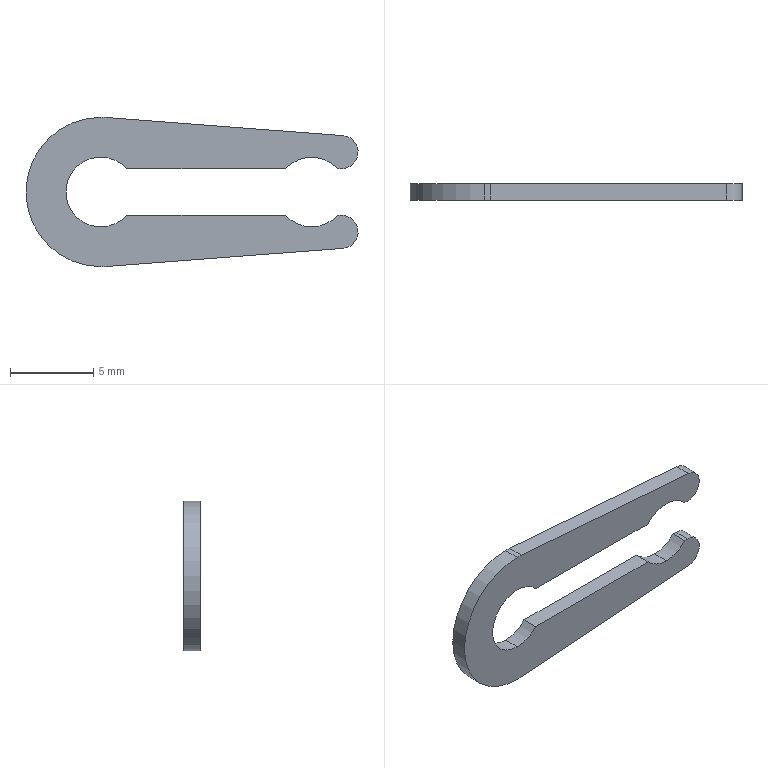Part | STEP file | 1 solid | 19 faces | box 20 x 1 x 9 mm | volume 97.65 mm3 | cylinder 11 | plane 8 | commonest cylinder face diameters 4.2 x6 9 x3 2 x2
STEP:
#1=CARTESIAN_POINT('',(0.,0.,0.));
#2=DIRECTION('',(0.,0.,1.));
#3=DIRECTION('',(1.,0.,0.));
#4=AXIS2_PLACEMENT_3D('',#1,#2,#3);
#5=CARTESIAN_POINT('',(7.915,1.,-1.4));
#6=VERTEX_POINT('',#5);
#7=CARTESIAN_POINT('',(7.915,0.,-1.4));
#8=VERTEX_POINT('',#7);
#9=CARTESIAN_POINT('',(7.915,1.,-1.4));
#10=DIRECTION('',(0.,-1.,0.));
#11=VECTOR('',#10,1.);
#12=LINE('',#9,#11);
#13=CARTESIAN_POINT('',(6.35,1.,0.));
#14=DIRECTION('',(0.,-1.,0.));
#15=DIRECTION('',(0.,0.,-1.));
#16=AXIS2_PLACEMENT_3D('',#13,#14,#15);
#17=CYLINDRICAL_SURFACE('',#16,2.1);
#18=CARTESIAN_POINT('',(0.8411,0.));
#19=DIRECTION('',(0.,1.));
#20=VECTOR('',#19,1.);
#21=LINE('',#18,#20);
#22=(GEOMETRIC_REPRESENTATION_CONTEXT(2)PARAMETRIC_REPRESENTATION_CONTEXT()REPRESENTATION_CONTEXT('',''));
#23=DEFINITIONAL_REPRESENTATION('',(#21),#22);
#24=PCURVE('',#17,#23);
#25=CARTESIAN_POINT('',(0.,1.,-1.4));
#26=DIRECTION('',(0.,0.,1.));
#27=DIRECTION('',(1.,0.,0.));
#28=AXIS2_PLACEMENT_3D('',#25,#26,#27);
#29=PLANE('',#28);
#30=CARTESIAN_POINT('',(7.915,0.));
#31=DIRECTION('',(0.,-1.));
#32=VECTOR('',#31,1.);
#33=LINE('',#30,#32);
#34=(GEOMETRIC_REPRESENTATION_CONTEXT(2)PARAMETRIC_REPRESENTATION_CONTEXT()REPRESENTATION_CONTEXT('',''));
#35=DEFINITIONAL_REPRESENTATION('',(#33),#34);
#36=PCURVE('',#29,#35);
#37=SURFACE_CURVE('',#12,(#24,#36),.PCURVE_S1.);
#38=EDGE_CURVE('',#6,#8,#37,.T.);
#39=ORIENTED_EDGE('',*,*,#38,.T.);
#40=CARTESIAN_POINT('',(6.35,0.,-2.1));
#41=VERTEX_POINT('',#40);
#42=CARTESIAN_POINT('',(6.35,0.,0.));
#43=DIRECTION('',(0.,-1.,0.));
#44=DIRECTION('',(0.,0.,1.));
#45=AXIS2_PLACEMENT_3D('',#42,#43,#44);
#46=CIRCLE('',#45,2.1);
#47=CARTESIAN_POINT('',(-3.142,1.));
#48=DIRECTION('',(1.,0.));
#49=VECTOR('',#48,1.);
#50=LINE('',#47,#49);
#51=(GEOMETRIC_REPRESENTATION_CONTEXT(2)PARAMETRIC_REPRESENTATION_CONTEXT()REPRESENTATION_CONTEXT('',''));
#52=DEFINITIONAL_REPRESENTATION('',(#50),#51);
#53=PCURVE('',#17,#52);
#54=CARTESIAN_POINT('',(0.,0.,0.));
#55=DIRECTION('',(0.,1.,0.));
#56=DIRECTION('',(0.,0.,1.));
#57=AXIS2_PLACEMENT_3D('',#54,#55,#56);
#58=PLANE('',#57);
#59=CARTESIAN_POINT('',(2.1,6.35));
#60=CARTESIAN_POINT('',(2.1,2.713));
#61=CARTESIAN_POINT('',(-1.05,4.531));
#62=CARTESIAN_POINT('',(-4.2,6.35));
#63=CARTESIAN_POINT('',(-1.05,8.169));
#64=CARTESIAN_POINT('',(2.1,9.987));
#65=CARTESIAN_POINT('',(2.1,6.35));
#66=(BOUNDED_CURVE()B_SPLINE_CURVE(2,(#59,#60,#61,#62,#63,#64,#65),.UNSPECIFIED.,.T.,.F.)B_SPLINE_CURVE_WITH_KNOTS((1,2,2,2,2,1),(-2.094,0.,2.094,4.189,6.283,8.378),.UNSPECIFIED.)CURVE()GEOMETRIC_REPRESENTATION_ITEM()RATIONAL_B_SPLINE_CURVE((1.,0.5,1.,0.5,1.,0.5,1.))REPRESENTATION_ITEM(''));
#67=(GEOMETRIC_REPRESENTATION_CONTEXT(2)PARAMETRIC_REPRESENTATION_CONTEXT()REPRESENTATION_CONTEXT('',''));
#68=DEFINITIONAL_REPRESENTATION('',(#66),#67);
#69=PCURVE('',#58,#68);
#70=SURFACE_CURVE('',#46,(#53,#69),.PCURVE_S1.);
#71=EDGE_CURVE('',#41,#8,#70,.T.);
#72=ORIENTED_EDGE('',*,*,#71,.F.);
#73=CARTESIAN_POINT('',(6.35,1.,-2.1));
#74=VERTEX_POINT('',#73);
#75=CARTESIAN_POINT('',(6.35,1.,-2.1));
#76=DIRECTION('',(0.,-1.,0.));
#77=VECTOR('',#76,1.);
#78=LINE('',#75,#77);
#79=CARTESIAN_POINT('',(0.,0.));
#80=DIRECTION('',(0.,1.));
#81=VECTOR('',#80,1.);
#82=LINE('',#79,#81);
#83=(GEOMETRIC_REPRESENTATION_CONTEXT(2)PARAMETRIC_REPRESENTATION_CONTEXT()REPRESENTATION_CONTEXT('',''));
#84=DEFINITIONAL_REPRESENTATION('',(#82),#83);
#85=PCURVE('',#17,#84);
#86=CARTESIAN_POINT('',(6.35,1.,0.));
#87=DIRECTION('',(0.,-1.,0.));
#88=DIRECTION('',(0.,0.,-1.));
#89=AXIS2_PLACEMENT_3D('',#86,#87,#88);
#90=CYLINDRICAL_SURFACE('',#89,2.1);
#91=CARTESIAN_POINT('',(6.283,0.));
#92=DIRECTION('',(0.,1.));
#93=VECTOR('',#92,1.);
#94=LINE('',#91,#93);
#95=(GEOMETRIC_REPRESENTATION_CONTEXT(2)PARAMETRIC_REPRESENTATION_CONTEXT()REPRESENTATION_CONTEXT('',''));
#96=DEFINITIONAL_REPRESENTATION('',(#94),#95);
#97=PCURVE('',#90,#96);
#98=SURFACE_CURVE('',#78,(#85,#97),.PCURVE_S1.);
#99=EDGE_CURVE('',#74,#41,#98,.T.);
#100=ORIENTED_EDGE('',*,*,#99,.F.);
#101=CARTESIAN_POINT('',(6.35,1.,0.));
#102=DIRECTION('',(0.,-1.,0.));
#103=DIRECTION('',(0.,0.,1.));
#104=AXIS2_PLACEMENT_3D('',#101,#102,#103);
#105=CIRCLE('',#104,2.1);
#106=CARTESIAN_POINT('',(-3.142,0.));
#107=DIRECTION('',(1.,0.));
#108=VECTOR('',#107,1.);
#109=LINE('',#106,#108);
#110=(GEOMETRIC_REPRESENTATION_CONTEXT(2)PARAMETRIC_REPRESENTATION_CONTEXT()REPRESENTATION_CONTEXT('',''));
#111=DEFINITIONAL_REPRESENTATION('',(#109),#110);
#112=PCURVE('',#17,#111);
#113=CARTESIAN_POINT('',(0.,1.,0.));
#114=DIRECTION('',(0.,1.,0.));
#115=DIRECTION('',(0.,0.,1.));
#116=AXIS2_PLACEMENT_3D('',#113,#114,#115);
#117=PLANE('',#116);
#118=CARTESIAN_POINT('',(2.1,6.35));
#119=CARTESIAN_POINT('',(2.1,2.713));
#120=CARTESIAN_POINT('',(-1.05,4.531));
#121=CARTESIAN_POINT('',(-4.2,6.35));
#122=CARTESIAN_POINT('',(-1.05,8.169));
#123=CARTESIAN_POINT('',(2.1,9.987));
#124=CARTESIAN_POINT('',(2.1,6.35));
#125=(BOUNDED_CURVE()B_SPLINE_CURVE(2,(#118,#119,#120,#121,#122,#123,#124),.UNSPECIFIED.,.T.,.F.)B_SPLINE_CURVE_WITH_KNOTS((1,2,2,2,2,1),(-2.094,0.,2.094,4.189,6.283,8.378),.UNSPECIFIED.)CURVE()GEOMETRIC_REPRESENTATION_ITEM()RATIONAL_B_SPLINE_CURVE((1.,0.5,1.,0.5,1.,0.5,1.))REPRESENTATION_ITEM(''));
#126=(GEOMETRIC_REPRESENTATION_CONTEXT(2)PARAMETRIC_REPRESENTATION_CONTEXT()REPRESENTATION_CONTEXT('',''));
#127=DEFINITIONAL_REPRESENTATION('',(#125),#126);
#128=PCURVE('',#117,#127);
#129=SURFACE_CURVE('',#105,(#112,#128),.PCURVE_S1.);
#130=EDGE_CURVE('',#74,#6,#129,.T.);
#131=ORIENTED_EDGE('',*,*,#130,.T.);
#132=EDGE_LOOP('',(#39,#72,#100,#131));
#133=FACE_BOUND('',#132,.F.);
#134=ADVANCED_FACE('',(#133),#17,.F.);
#135=CARTESIAN_POINT('',(-6.35,1.,-2.1));
#136=VERTEX_POINT('',#135);
#137=CARTESIAN_POINT('',(-6.35,0.,-2.1));
#138=VERTEX_POINT('',#137);
#139=CARTESIAN_POINT('',(-6.35,1.,-2.1));
#140=DIRECTION('',(0.,-1.,0.));
#141=VECTOR('',#140,1.);
#142=LINE('',#139,#141);
#143=CARTESIAN_POINT('',(-6.35,1.,0.));
#144=DIRECTION('',(0.,-1.,0.));
#145=DIRECTION('',(0.,0.,-1.));
#146=AXIS2_PLACEMENT_3D('',#143,#144,#145);
#147=CYLINDRICAL_SURFACE('',#146,2.1);
#148=CARTESIAN_POINT('',(6.283,0.));
#149=DIRECTION('',(0.,1.));
#150=VECTOR('',#149,1.);
#151=LINE('',#148,#150);
#152=(GEOMETRIC_REPRESENTATION_CONTEXT(2)PARAMETRIC_REPRESENTATION_CONTEXT()REPRESENTATION_CONTEXT('',''));
#153=DEFINITIONAL_REPRESENTATION('',(#151),#152);
#154=PCURVE('',#147,#153);
#155=CARTESIAN_POINT('',(-6.35,1.,0.));
#156=DIRECTION('',(0.,-1.,0.));
#157=DIRECTION('',(0.,0.,-1.));
#158=AXIS2_PLACEMENT_3D('',#155,#156,#157);
#159=CYLINDRICAL_SURFACE('',#158,2.1);
#160=CARTESIAN_POINT('',(0.,0.));
#161=DIRECTION('',(0.,1.));
#162=VECTOR('',#161,1.);
#163=LINE('',#160,#162);
#164=(GEOMETRIC_REPRESENTATION_CONTEXT(2)PARAMETRIC_REPRESENTATION_CONTEXT()REPRESENTATION_CONTEXT('',''));
#165=DEFINITIONAL_REPRESENTATION('',(#163),#164);
#166=PCURVE('',#159,#165);
#167=SURFACE_CURVE('',#142,(#154,#166),.PCURVE_S1.);
#168=EDGE_CURVE('',#136,#138,#167,.T.);
#169=ORIENTED_EDGE('',*,*,#168,.T.);
#170=CARTESIAN_POINT('',(-6.35,0.,2.1));
#171=VERTEX_POINT('',#170);
#172=CARTESIAN_POINT('',(-6.35,0.,0.));
#173=DIRECTION('',(0.,1.,0.));
#174=DIRECTION('',(0.,0.,1.));
#175=AXIS2_PLACEMENT_3D('',#172,#173,#174);
#176=CIRCLE('',#175,2.1);
#177=CARTESIAN_POINT('',(9.425,1.));
#178=DIRECTION('',(-1.,0.));
#179=VECTOR('',#178,1.);
#180=LINE('',#177,#179);
#181=(GEOMETRIC_REPRESENTATION_CONTEXT(2)PARAMETRIC_REPRESENTATION_CONTEXT()REPRESENTATION_CONTEXT('',''));
#182=DEFINITIONAL_REPRESENTATION('',(#180),#181);
#183=PCURVE('',#147,#182);
#184=CARTESIAN_POINT('',(0.,-6.35));
#185=DIRECTION('',(1.,0.));
#186=AXIS2_PLACEMENT_2D('',#184,#185);
#187=CIRCLE('',#186,2.1);
#188=(GEOMETRIC_REPRESENTATION_CONTEXT(2)PARAMETRIC_REPRESENTATION_CONTEXT()REPRESENTATION_CONTEXT('',''));
#189=DEFINITIONAL_REPRESENTATION('',(#187),#188);
#190=PCURVE('',#58,#189);
#191=SURFACE_CURVE('',#176,(#183,#190),.PCURVE_S1.);
#192=EDGE_CURVE('',#138,#171,#191,.T.);
#193=ORIENTED_EDGE('',*,*,#192,.T.);
#194=CARTESIAN_POINT('',(-6.35,1.,2.1));
#195=VERTEX_POINT('',#194);
#196=CARTESIAN_POINT('',(-6.35,1.,2.1));
#197=DIRECTION('',(0.,-1.,0.));
#198=VECTOR('',#197,1.);
#199=LINE('',#196,#198);
#200=CARTESIAN_POINT('',(3.142,0.));
#201=DIRECTION('',(0.,1.));
#202=VECTOR('',#201,1.);
#203=LINE('',#200,#202);
#204=(GEOMETRIC_REPRESENTATION_CONTEXT(2)PARAMETRIC_REPRESENTATION_CONTEXT()REPRESENTATION_CONTEXT('',''));
#205=DEFINITIONAL_REPRESENTATION('',(#203),#204);
#206=PCURVE('',#147,#205);
#207=CARTESIAN_POINT('',(-6.35,1.,0.));
#208=DIRECTION('',(0.,-1.,0.));
#209=DIRECTION('',(0.,0.,-1.));
#210=AXIS2_PLACEMENT_3D('',#207,#208,#209);
#211=CYLINDRICAL_SURFACE('',#210,2.1);
#212=CARTESIAN_POINT('',(3.142,0.));
#213=DIRECTION('',(0.,1.));
#214=VECTOR('',#213,1.);
#215=LINE('',#212,#214);
#216=(GEOMETRIC_REPRESENTATION_CONTEXT(2)PARAMETRIC_REPRESENTATION_CONTEXT()REPRESENTATION_CONTEXT('',''));
#217=DEFINITIONAL_REPRESENTATION('',(#215),#216);
#218=PCURVE('',#211,#217);
#219=SURFACE_CURVE('',#199,(#206,#218),.PCURVE_S1.);
#220=EDGE_CURVE('',#195,#171,#219,.T.);
#221=ORIENTED_EDGE('',*,*,#220,.F.);
#222=CARTESIAN_POINT('',(-6.35,1.,0.));
#223=DIRECTION('',(0.,1.,0.));
#224=DIRECTION('',(0.,0.,1.));
#225=AXIS2_PLACEMENT_3D('',#222,#223,#224);
#226=CIRCLE('',#225,2.1);
#227=CARTESIAN_POINT('',(9.425,0.));
#228=DIRECTION('',(-1.,0.));
#229=VECTOR('',#228,1.);
#230=LINE('',#227,#229);
#231=(GEOMETRIC_REPRESENTATION_CONTEXT(2)PARAMETRIC_REPRESENTATION_CONTEXT()REPRESENTATION_CONTEXT('',''));
#232=DEFINITIONAL_REPRESENTATION('',(#230),#231);
#233=PCURVE('',#147,#232);
#234=CARTESIAN_POINT('',(0.,-6.35));
#235=DIRECTION('',(1.,0.));
#236=AXIS2_PLACEMENT_2D('',#234,#235);
#237=CIRCLE('',#236,2.1);
#238=(GEOMETRIC_REPRESENTATION_CONTEXT(2)PARAMETRIC_REPRESENTATION_CONTEXT()REPRESENTATION_CONTEXT('',''));
#239=DEFINITIONAL_REPRESENTATION('',(#237),#238);
#240=PCURVE('',#117,#239);
#241=SURFACE_CURVE('',#226,(#233,#240),.PCURVE_S1.);
#242=EDGE_CURVE('',#136,#195,#241,.T.);
#243=ORIENTED_EDGE('',*,*,#242,.F.);
#244=EDGE_LOOP('',(#169,#193,#221,#243));
#245=FACE_BOUND('',#244,.F.);
#246=ADVANCED_FACE('',(#245),#147,.F.);
#247=CARTESIAN_POINT('',(-4.785,1.,-1.4));
#248=VERTEX_POINT('',#247);
#249=CARTESIAN_POINT('',(-4.785,0.,-1.4));
#250=VERTEX_POINT('',#249);
#251=CARTESIAN_POINT('',(-4.785,1.,-1.4));
#252=DIRECTION('',(0.,-1.,0.));
#253=VECTOR('',#252,1.);
#254=LINE('',#251,#253);
#255=CARTESIAN_POINT('',(0.8411,0.));
#256=DIRECTION('',(0.,1.));
#257=VECTOR('',#256,1.);
#258=LINE('',#255,#257);
#259=(GEOMETRIC_REPRESENTATION_CONTEXT(2)PARAMETRIC_REPRESENTATION_CONTEXT()REPRESENTATION_CONTEXT('',''));
#260=DEFINITIONAL_REPRESENTATION('',(#258),#259);
#261=PCURVE('',#159,#260);
#262=CARTESIAN_POINT('',(0.,1.,-1.4));
#263=DIRECTION('',(0.,0.,1.));
#264=DIRECTION('',(1.,0.,0.));
#265=AXIS2_PLACEMENT_3D('',#262,#263,#264);
#266=PLANE('',#265);
#267=CARTESIAN_POINT('',(-4.785,0.));
#268=DIRECTION('',(0.,-1.));
#269=VECTOR('',#268,1.);
#270=LINE('',#267,#269);
#271=(GEOMETRIC_REPRESENTATION_CONTEXT(2)PARAMETRIC_REPRESENTATION_CONTEXT()REPRESENTATION_CONTEXT('',''));
#272=DEFINITIONAL_REPRESENTATION('',(#270),#271);
#273=PCURVE('',#266,#272);
#274=SURFACE_CURVE('',#254,(#261,#273),.PCURVE_S1.);
#275=EDGE_CURVE('',#248,#250,#274,.T.);
#276=ORIENTED_EDGE('',*,*,#275,.T.);
#277=CARTESIAN_POINT('',(-6.35,0.,0.));
#278=DIRECTION('',(0.,1.,0.));
#279=DIRECTION('',(0.,0.,1.));
#280=AXIS2_PLACEMENT_3D('',#277,#278,#279);
#281=CIRCLE('',#280,2.1);
#282=CARTESIAN_POINT('',(3.142,1.));
#283=DIRECTION('',(-1.,0.));
#284=VECTOR('',#283,1.);
#285=LINE('',#282,#284);
#286=(GEOMETRIC_REPRESENTATION_CONTEXT(2)PARAMETRIC_REPRESENTATION_CONTEXT()REPRESENTATION_CONTEXT('',''));
#287=DEFINITIONAL_REPRESENTATION('',(#285),#286);
#288=PCURVE('',#159,#287);
#289=CARTESIAN_POINT('',(0.,-6.35));
#290=DIRECTION('',(1.,0.));
#291=AXIS2_PLACEMENT_2D('',#289,#290);
#292=CIRCLE('',#291,2.1);
#293=(GEOMETRIC_REPRESENTATION_CONTEXT(2)PARAMETRIC_REPRESENTATION_CONTEXT()REPRESENTATION_CONTEXT('',''));
#294=DEFINITIONAL_REPRESENTATION('',(#292),#293);
#295=PCURVE('',#58,#294);
#296=SURFACE_CURVE('',#281,(#288,#295),.PCURVE_S1.);
#297=EDGE_CURVE('',#250,#138,#296,.T.);
#298=ORIENTED_EDGE('',*,*,#297,.T.);
#299=ORIENTED_EDGE('',*,*,#168,.F.);
#300=CARTESIAN_POINT('',(-6.35,1.,0.));
#301=DIRECTION('',(0.,1.,0.));
#302=DIRECTION('',(0.,0.,1.));
#303=AXIS2_PLACEMENT_3D('',#300,#301,#302);
#304=CIRCLE('',#303,2.1);
#305=CARTESIAN_POINT('',(3.142,0.));
#306=DIRECTION('',(-1.,0.));
#307=VECTOR('',#306,1.);
#308=LINE('',#305,#307);
#309=(GEOMETRIC_REPRESENTATION_CONTEXT(2)PARAMETRIC_REPRESENTATION_CONTEXT()REPRESENTATION_CONTEXT('',''));
#310=DEFINITIONAL_REPRESENTATION('',(#308),#309);
#311=PCURVE('',#159,#310);
#312=CARTESIAN_POINT('',(0.,-6.35));
#313=DIRECTION('',(1.,0.));
#314=AXIS2_PLACEMENT_2D('',#312,#313);
#315=CIRCLE('',#314,2.1);
#316=(GEOMETRIC_REPRESENTATION_CONTEXT(2)PARAMETRIC_REPRESENTATION_CONTEXT()REPRESENTATION_CONTEXT('',''));
#317=DEFINITIONAL_REPRESENTATION('',(#315),#316);
#318=PCURVE('',#117,#317);
#319=SURFACE_CURVE('',#304,(#311,#318),.PCURVE_S1.);
#320=EDGE_CURVE('',#248,#136,#319,.T.);
#321=ORIENTED_EDGE('',*,*,#320,.F.);
#322=EDGE_LOOP('',(#276,#298,#299,#321));
#323=FACE_BOUND('',#322,.F.);
#324=ADVANCED_FACE('',(#323),#159,.F.);
#325=CARTESIAN_POINT('',(-6.35,1.,4.5));
#326=VERTEX_POINT('',#325);
#327=CARTESIAN_POINT('',(-6.006,1.,4.487));
#328=VERTEX_POINT('',#327);
#329=CARTESIAN_POINT('',(-6.35,1.,0.));
#330=DIRECTION('',(0.,1.,0.));
#331=DIRECTION('',(0.,0.,1.));
#332=AXIS2_PLACEMENT_3D('',#329,#330,#331);
#333=CIRCLE('',#332,4.5);
#334=CARTESIAN_POINT('',(-6.35,1.,0.));
#335=DIRECTION('',(0.,-1.,0.));
#336=DIRECTION('',(0.,0.,-1.));
#337=AXIS2_PLACEMENT_3D('',#334,#335,#336);
#338=CYLINDRICAL_SURFACE('',#337,4.5);
#339=CARTESIAN_POINT('',(3.142,0.));
#340=DIRECTION('',(-1.,0.));
#341=VECTOR('',#340,1.);
#342=LINE('',#339,#341);
#343=(GEOMETRIC_REPRESENTATION_CONTEXT(2)PARAMETRIC_REPRESENTATION_CONTEXT()REPRESENTATION_CONTEXT('',''));
#344=DEFINITIONAL_REPRESENTATION('',(#342),#343);
#345=PCURVE('',#338,#344);
#346=CARTESIAN_POINT('',(0.,-6.35));
#347=DIRECTION('',(1.,0.));
#348=AXIS2_PLACEMENT_2D('',#346,#347);
#349=CIRCLE('',#348,4.5);
#350=(GEOMETRIC_REPRESENTATION_CONTEXT(2)PARAMETRIC_REPRESENTATION_CONTEXT()REPRESENTATION_CONTEXT('',''));
#351=DEFINITIONAL_REPRESENTATION('',(#349),#350);
#352=PCURVE('',#117,#351);
#353=SURFACE_CURVE('',#333,(#345,#352),.PCURVE_S1.);
#354=EDGE_CURVE('',#326,#328,#353,.T.);
#355=ORIENTED_EDGE('',*,*,#354,.F.);
#356=CARTESIAN_POINT('',(-6.35,0.,4.5));
#357=VERTEX_POINT('',#356);
#358=CARTESIAN_POINT('',(-6.35,1.,4.5));
#359=DIRECTION('',(0.,-1.,0.));
#360=VECTOR('',#359,1.);
#361=LINE('',#358,#360);
#362=CARTESIAN_POINT('',(3.142,0.));
#363=DIRECTION('',(0.,1.));
#364=VECTOR('',#363,1.);
#365=LINE('',#362,#364);
#366=(GEOMETRIC_REPRESENTATION_CONTEXT(2)PARAMETRIC_REPRESENTATION_CONTEXT()REPRESENTATION_CONTEXT('',''));
#367=DEFINITIONAL_REPRESENTATION('',(#365),#366);
#368=PCURVE('',#338,#367);
#369=CARTESIAN_POINT('',(-6.35,1.,0.));
#370=DIRECTION('',(0.,-1.,0.));
#371=DIRECTION('',(0.,0.,-1.));
#372=AXIS2_PLACEMENT_3D('',#369,#370,#371);
#373=CYLINDRICAL_SURFACE('',#372,4.5);
#374=CARTESIAN_POINT('',(3.142,0.));
#375=DIRECTION('',(0.,1.));
#376=VECTOR('',#375,1.);
#377=LINE('',#374,#376);
#378=(GEOMETRIC_REPRESENTATION_CONTEXT(2)PARAMETRIC_REPRESENTATION_CONTEXT()REPRESENTATION_CONTEXT('',''));
#379=DEFINITIONAL_REPRESENTATION('',(#377),#378);
#380=PCURVE('',#373,#379);
#381=SURFACE_CURVE('',#361,(#368,#380),.PCURVE_S1.);
#382=EDGE_CURVE('',#326,#357,#381,.T.);
#383=ORIENTED_EDGE('',*,*,#382,.T.);
#384=CARTESIAN_POINT('',(-6.006,0.,4.487));
#385=VERTEX_POINT('',#384);
#386=CARTESIAN_POINT('',(-6.35,0.,0.));
#387=DIRECTION('',(0.,1.,0.));
#388=DIRECTION('',(0.,0.,1.));
#389=AXIS2_PLACEMENT_3D('',#386,#387,#388);
#390=CIRCLE('',#389,4.5);
#391=CARTESIAN_POINT('',(3.142,1.));
#392=DIRECTION('',(-1.,0.));
#393=VECTOR('',#392,1.);
#394=LINE('',#391,#393);
#395=(GEOMETRIC_REPRESENTATION_CONTEXT(2)PARAMETRIC_REPRESENTATION_CONTEXT()REPRESENTATION_CONTEXT('',''));
#396=DEFINITIONAL_REPRESENTATION('',(#394),#395);
#397=PCURVE('',#338,#396);
#398=CARTESIAN_POINT('',(0.,-6.35));
#399=DIRECTION('',(1.,0.));
#400=AXIS2_PLACEMENT_2D('',#398,#399);
#401=CIRCLE('',#400,4.5);
#402=(GEOMETRIC_REPRESENTATION_CONTEXT(2)PARAMETRIC_REPRESENTATION_CONTEXT()REPRESENTATION_CONTEXT('',''));
#403=DEFINITIONAL_REPRESENTATION('',(#401),#402);
#404=PCURVE('',#58,#403);
#405=SURFACE_CURVE('',#390,(#397,#404),.PCURVE_S1.);
#406=EDGE_CURVE('',#357,#385,#405,.T.);
#407=ORIENTED_EDGE('',*,*,#406,.T.);
#408=CARTESIAN_POINT('',(-6.006,1.,4.487));
#409=DIRECTION('',(0.,-1.,0.));
#410=VECTOR('',#409,1.);
#411=LINE('',#408,#410);
#412=CARTESIAN_POINT('',(3.065,0.));
#413=DIRECTION('',(0.,1.));
#414=VECTOR('',#413,1.);
#415=LINE('',#412,#414);
#416=(GEOMETRIC_REPRESENTATION_CONTEXT(2)PARAMETRIC_REPRESENTATION_CONTEXT()REPRESENTATION_CONTEXT('',''));
#417=DEFINITIONAL_REPRESENTATION('',(#415),#416);
#418=PCURVE('',#338,#417);
#419=CARTESIAN_POINT('',(0.3065,1.,4.003));
#420=DIRECTION('',(-0.07635,0.,-0.9971));
#421=DIRECTION('',(-0.9971,0.,0.07635));
#422=AXIS2_PLACEMENT_3D('',#419,#420,#421);
#423=PLANE('',#422);
#424=CARTESIAN_POINT('',(6.331,0.));
#425=DIRECTION('',(0.,-1.));
#426=VECTOR('',#425,1.);
#427=LINE('',#424,#426);
#428=(GEOMETRIC_REPRESENTATION_CONTEXT(2)PARAMETRIC_REPRESENTATION_CONTEXT()REPRESENTATION_CONTEXT('',''));
#429=DEFINITIONAL_REPRESENTATION('',(#427),#428);
#430=PCURVE('',#423,#429);
#431=SURFACE_CURVE('',#411,(#418,#430),.PCURVE_S1.);
#432=EDGE_CURVE('',#328,#385,#431,.T.);
#433=ORIENTED_EDGE('',*,*,#432,.F.);
#434=EDGE_LOOP('',(#355,#383,#407,#433));
#435=FACE_BOUND('',#434,.T.);
#436=ADVANCED_FACE('',(#435),#338,.T.);
#437=ORIENTED_EDGE('',*,*,#382,.F.);
#438=CARTESIAN_POINT('',(-6.35,1.,-4.5));
#439=VERTEX_POINT('',#438);
#440=CARTESIAN_POINT('',(-6.35,1.,0.));
#441=DIRECTION('',(0.,1.,0.));
#442=DIRECTION('',(0.,0.,1.));
#443=AXIS2_PLACEMENT_3D('',#440,#441,#442);
#444=CIRCLE('',#443,4.5);
#445=CARTESIAN_POINT('',(9.425,0.));
#446=DIRECTION('',(-1.,0.));
#447=VECTOR('',#446,1.);
#448=LINE('',#445,#447);
#449=(GEOMETRIC_REPRESENTATION_CONTEXT(2)PARAMETRIC_REPRESENTATION_CONTEXT()REPRESENTATION_CONTEXT('',''));
#450=DEFINITIONAL_REPRESENTATION('',(#448),#449);
#451=PCURVE('',#373,#450);
#452=CARTESIAN_POINT('',(0.,-6.35));
#453=DIRECTION('',(1.,0.));
#454=AXIS2_PLACEMENT_2D('',#452,#453);
#455=CIRCLE('',#454,4.5);
#456=(GEOMETRIC_REPRESENTATION_CONTEXT(2)PARAMETRIC_REPRESENTATION_CONTEXT()REPRESENTATION_CONTEXT('',''));
#457=DEFINITIONAL_REPRESENTATION('',(#455),#456);
#458=PCURVE('',#117,#457);
#459=SURFACE_CURVE('',#444,(#451,#458),.PCURVE_S1.);
#460=EDGE_CURVE('',#439,#326,#459,.T.);
#461=ORIENTED_EDGE('',*,*,#460,.F.);
#462=CARTESIAN_POINT('',(-6.35,0.,-4.5));
#463=VERTEX_POINT('',#462);
#464=CARTESIAN_POINT('',(-6.35,1.,-4.5));
#465=DIRECTION('',(0.,-1.,0.));
#466=VECTOR('',#465,1.);
#467=LINE('',#464,#466);
#468=CARTESIAN_POINT('',(6.283,0.));
#469=DIRECTION('',(0.,1.));
#470=VECTOR('',#469,1.);
#471=LINE('',#468,#470);
#472=(GEOMETRIC_REPRESENTATION_CONTEXT(2)PARAMETRIC_REPRESENTATION_CONTEXT()REPRESENTATION_CONTEXT('',''));
#473=DEFINITIONAL_REPRESENTATION('',(#471),#472);
#474=PCURVE('',#373,#473);
#475=CARTESIAN_POINT('',(-6.35,1.,0.));
#476=DIRECTION('',(0.,-1.,0.));
#477=DIRECTION('',(0.,0.,-1.));
#478=AXIS2_PLACEMENT_3D('',#475,#476,#477);
#479=CYLINDRICAL_SURFACE('',#478,4.5);
#480=CARTESIAN_POINT('',(0.,0.));
#481=DIRECTION('',(0.,1.));
#482=VECTOR('',#481,1.);
#483=LINE('',#480,#482);
#484=(GEOMETRIC_REPRESENTATION_CONTEXT(2)PARAMETRIC_REPRESENTATION_CONTEXT()REPRESENTATION_CONTEXT('',''));
#485=DEFINITIONAL_REPRESENTATION('',(#483),#484);
#486=PCURVE('',#479,#485);
#487=SURFACE_CURVE('',#467,(#474,#486),.PCURVE_S1.);
#488=EDGE_CURVE('',#439,#463,#487,.T.);
#489=ORIENTED_EDGE('',*,*,#488,.T.);
#490=CARTESIAN_POINT('',(-6.35,0.,0.));
#491=DIRECTION('',(0.,1.,0.));
#492=DIRECTION('',(0.,0.,1.));
#493=AXIS2_PLACEMENT_3D('',#490,#491,#492);
#494=CIRCLE('',#493,4.5);
#495=CARTESIAN_POINT('',(9.425,1.));
#496=DIRECTION('',(-1.,0.));
#497=VECTOR('',#496,1.);
#498=LINE('',#495,#497);
#499=(GEOMETRIC_REPRESENTATION_CONTEXT(2)PARAMETRIC_REPRESENTATION_CONTEXT()REPRESENTATION_CONTEXT('',''));
#500=DEFINITIONAL_REPRESENTATION('',(#498),#499);
#501=PCURVE('',#373,#500);
#502=CARTESIAN_POINT('',(0.,-6.35));
#503=DIRECTION('',(1.,0.));
#504=AXIS2_PLACEMENT_2D('',#502,#503);
#505=CIRCLE('',#504,4.5);
#506=(GEOMETRIC_REPRESENTATION_CONTEXT(2)PARAMETRIC_REPRESENTATION_CONTEXT()REPRESENTATION_CONTEXT('',''));
#507=DEFINITIONAL_REPRESENTATION('',(#505),#506);
#508=PCURVE('',#58,#507);
#509=SURFACE_CURVE('',#494,(#501,#508),.PCURVE_S1.);
#510=EDGE_CURVE('',#463,#357,#509,.T.);
#511=ORIENTED_EDGE('',*,*,#510,.T.);
#512=EDGE_LOOP('',(#437,#461,#489,#511));
#513=FACE_BOUND('',#512,.T.);
#514=ADVANCED_FACE('',(#513),#373,.T.);
#515=CARTESIAN_POINT('',(-6.006,0.,-4.487));
#516=VERTEX_POINT('',#515);
#517=CARTESIAN_POINT('',(8.226,0.,-3.397));
#518=VERTEX_POINT('',#517);
#519=CARTESIAN_POINT('',(0.3065,0.,-4.003));
#520=DIRECTION('',(0.9971,0.,0.07635));
#521=VECTOR('',#520,1.);
#522=LINE('',#519,#521);
#523=CARTESIAN_POINT('',(0.3065,1.,-4.003));
#524=DIRECTION('',(0.07635,0.,-0.9971));
#525=DIRECTION('',(-0.9971,0.,-0.07635));
#526=AXIS2_PLACEMENT_3D('',#523,#524,#525);
#527=PLANE('',#526);
#528=CARTESIAN_POINT('',(0.,-1.));
#529=DIRECTION('',(-1.,0.));
#530=VECTOR('',#529,1.);
#531=LINE('',#528,#530);
#532=(GEOMETRIC_REPRESENTATION_CONTEXT(2)PARAMETRIC_REPRESENTATION_CONTEXT()REPRESENTATION_CONTEXT('',''));
#533=DEFINITIONAL_REPRESENTATION('',(#531),#532);
#534=PCURVE('',#527,#533);
#535=CARTESIAN_POINT('',(-4.003,0.3065));
#536=DIRECTION('',(0.07635,0.9971));
#537=VECTOR('',#536,1.);
#538=LINE('',#535,#537);
#539=(GEOMETRIC_REPRESENTATION_CONTEXT(2)PARAMETRIC_REPRESENTATION_CONTEXT()REPRESENTATION_CONTEXT('',''));
#540=DEFINITIONAL_REPRESENTATION('',(#538),#539);
#541=PCURVE('',#58,#540);
#542=SURFACE_CURVE('',#522,(#534,#541),.PCURVE_S1.);
#543=EDGE_CURVE('',#516,#518,#542,.T.);
#544=ORIENTED_EDGE('',*,*,#543,.F.);
#545=CARTESIAN_POINT('',(-6.006,1.,-4.487));
#546=VERTEX_POINT('',#545);
#547=CARTESIAN_POINT('',(-6.006,1.,-4.487));
#548=DIRECTION('',(0.,-1.,0.));
#549=VECTOR('',#548,1.);
#550=LINE('',#547,#549);
#551=CARTESIAN_POINT('',(6.331,0.));
#552=DIRECTION('',(0.,-1.));
#553=VECTOR('',#552,1.);
#554=LINE('',#551,#553);
#555=(GEOMETRIC_REPRESENTATION_CONTEXT(2)PARAMETRIC_REPRESENTATION_CONTEXT()REPRESENTATION_CONTEXT('',''));
#556=DEFINITIONAL_REPRESENTATION('',(#554),#555);
#557=PCURVE('',#527,#556);
#558=CARTESIAN_POINT('',(0.07642,0.));
#559=DIRECTION('',(0.,1.));
#560=VECTOR('',#559,1.);
#561=LINE('',#558,#560);
#562=(GEOMETRIC_REPRESENTATION_CONTEXT(2)PARAMETRIC_REPRESENTATION_CONTEXT()REPRESENTATION_CONTEXT('',''));
#563=DEFINITIONAL_REPRESENTATION('',(#561),#562);
#564=PCURVE('',#479,#563);
#565=SURFACE_CURVE('',#550,(#557,#564),.PCURVE_S1.);
#566=EDGE_CURVE('',#546,#516,#565,.T.);
#567=ORIENTED_EDGE('',*,*,#566,.F.);
#568=CARTESIAN_POINT('',(8.226,1.,-3.397));
#569=VERTEX_POINT('',#568);
#570=CARTESIAN_POINT('',(0.3065,1.,-4.003));
#571=DIRECTION('',(0.9971,0.,0.07635));
#572=VECTOR('',#571,1.);
#573=LINE('',#570,#572);
#574=CARTESIAN_POINT('',(0.,0.));
#575=DIRECTION('',(-1.,0.));
#576=VECTOR('',#575,1.);
#577=LINE('',#574,#576);
#578=(GEOMETRIC_REPRESENTATION_CONTEXT(2)PARAMETRIC_REPRESENTATION_CONTEXT()REPRESENTATION_CONTEXT('',''));
#579=DEFINITIONAL_REPRESENTATION('',(#577),#578);
#580=PCURVE('',#527,#579);
#581=CARTESIAN_POINT('',(-4.003,0.3065));
#582=DIRECTION('',(0.07635,0.9971));
#583=VECTOR('',#582,1.);
#584=LINE('',#581,#583);
#585=(GEOMETRIC_REPRESENTATION_CONTEXT(2)PARAMETRIC_REPRESENTATION_CONTEXT()REPRESENTATION_CONTEXT('',''));
#586=DEFINITIONAL_REPRESENTATION('',(#584),#585);
#587=PCURVE('',#117,#586);
#588=SURFACE_CURVE('',#573,(#580,#587),.PCURVE_S1.);
#589=EDGE_CURVE('',#546,#569,#588,.T.);
#590=ORIENTED_EDGE('',*,*,#589,.T.);
#591=CARTESIAN_POINT('',(8.226,1.,-3.397));
#592=DIRECTION('',(0.,-1.,0.));
#593=VECTOR('',#592,1.);
#594=LINE('',#591,#593);
#595=CARTESIAN_POINT('',(-7.943,0.));
#596=DIRECTION('',(0.,-1.));
#597=VECTOR('',#596,1.);
#598=LINE('',#595,#597);
#599=(GEOMETRIC_REPRESENTATION_CONTEXT(2)PARAMETRIC_REPRESENTATION_CONTEXT()REPRESENTATION_CONTEXT('',''));
#600=DEFINITIONAL_REPRESENTATION('',(#598),#599);
#601=PCURVE('',#527,#600);
#602=CARTESIAN_POINT('',(8.15,1.,-2.4));
#603=DIRECTION('',(0.,-1.,0.));
#604=DIRECTION('',(0.,0.,-1.));
#605=AXIS2_PLACEMENT_3D('',#602,#603,#604);
#606=CYLINDRICAL_SURFACE('',#605,1.);
#607=CARTESIAN_POINT('',(0.07642,0.));
#608=DIRECTION('',(0.,1.));
#609=VECTOR('',#608,1.);
#610=LINE('',#607,#609);
#611=(GEOMETRIC_REPRESENTATION_CONTEXT(2)PARAMETRIC_REPRESENTATION_CONTEXT()REPRESENTATION_CONTEXT('',''));
#612=DEFINITIONAL_REPRESENTATION('',(#610),#611);
#613=PCURVE('',#606,#612);
#614=SURFACE_CURVE('',#594,(#601,#613),.PCURVE_S1.);
#615=EDGE_CURVE('',#569,#518,#614,.T.);
#616=ORIENTED_EDGE('',*,*,#615,.T.);
#617=EDGE_LOOP('',(#544,#567,#590,#616));
#618=FACE_BOUND('',#617,.T.);
#619=ADVANCED_FACE('',(#618),#527,.T.);
#620=ORIENTED_EDGE('',*,*,#488,.F.);
#621=CARTESIAN_POINT('',(-6.35,1.,0.));
#622=DIRECTION('',(0.,1.,0.));
#623=DIRECTION('',(0.,0.,1.));
#624=AXIS2_PLACEMENT_3D('',#621,#622,#623);
#625=CIRCLE('',#624,4.5);
#626=CARTESIAN_POINT('',(3.142,0.));
#627=DIRECTION('',(-1.,0.));
#628=VECTOR('',#627,1.);
#629=LINE('',#626,#628);
#630=(GEOMETRIC_REPRESENTATION_CONTEXT(2)PARAMETRIC_REPRESENTATION_CONTEXT()REPRESENTATION_CONTEXT('',''));
#631=DEFINITIONAL_REPRESENTATION('',(#629),#630);
#632=PCURVE('',#479,#631);
#633=CARTESIAN_POINT('',(0.,-6.35));
#634=DIRECTION('',(1.,0.));
#635=AXIS2_PLACEMENT_2D('',#633,#634);
#636=CIRCLE('',#635,4.5);
#637=(GEOMETRIC_REPRESENTATION_CONTEXT(2)PARAMETRIC_REPRESENTATION_CONTEXT()REPRESENTATION_CONTEXT('',''));
#638=DEFINITIONAL_REPRESENTATION('',(#636),#637);
#639=PCURVE('',#117,#638);
#640=SURFACE_CURVE('',#625,(#632,#639),.PCURVE_S1.);
#641=EDGE_CURVE('',#546,#439,#640,.T.);
#642=ORIENTED_EDGE('',*,*,#641,.F.);
#643=ORIENTED_EDGE('',*,*,#566,.T.);
#644=CARTESIAN_POINT('',(-6.35,0.,0.));
#645=DIRECTION('',(0.,1.,0.));
#646=DIRECTION('',(0.,0.,1.));
#647=AXIS2_PLACEMENT_3D('',#644,#645,#646);
#648=CIRCLE('',#647,4.5);
#649=CARTESIAN_POINT('',(3.142,1.));
#650=DIRECTION('',(-1.,0.));
#651=VECTOR('',#650,1.);
#652=LINE('',#649,#651);
#653=(GEOMETRIC_REPRESENTATION_CONTEXT(2)PARAMETRIC_REPRESENTATION_CONTEXT()REPRESENTATION_CONTEXT('',''));
#654=DEFINITIONAL_REPRESENTATION('',(#652),#653);
#655=PCURVE('',#479,#654);
#656=CARTESIAN_POINT('',(0.,-6.35));
#657=DIRECTION('',(1.,0.));
#658=AXIS2_PLACEMENT_2D('',#656,#657);
#659=CIRCLE('',#658,4.5);
#660=(GEOMETRIC_REPRESENTATION_CONTEXT(2)PARAMETRIC_REPRESENTATION_CONTEXT()REPRESENTATION_CONTEXT('',''));
#661=DEFINITIONAL_REPRESENTATION('',(#659),#660);
#662=PCURVE('',#58,#661);
#663=SURFACE_CURVE('',#648,(#655,#662),.PCURVE_S1.);
#664=EDGE_CURVE('',#516,#463,#663,.T.);
#665=ORIENTED_EDGE('',*,*,#664,.T.);
#666=EDGE_LOOP('',(#620,#642,#643,#665));
#667=FACE_BOUND('',#666,.T.);
#668=ADVANCED_FACE('',(#667),#479,.T.);
#669=CARTESIAN_POINT('',(8.226,0.,3.397));
#670=VERTEX_POINT('',#669);
#671=CARTESIAN_POINT('',(0.3065,0.,4.003));
#672=DIRECTION('',(0.9971,0.,-0.07635));
#673=VECTOR('',#672,1.);
#674=LINE('',#671,#673);
#675=CARTESIAN_POINT('',(0.,-1.));
#676=DIRECTION('',(-1.,0.));
#677=VECTOR('',#676,1.);
#678=LINE('',#675,#677);
#679=(GEOMETRIC_REPRESENTATION_CONTEXT(2)PARAMETRIC_REPRESENTATION_CONTEXT()REPRESENTATION_CONTEXT('',''));
#680=DEFINITIONAL_REPRESENTATION('',(#678),#679);
#681=PCURVE('',#423,#680);
#682=CARTESIAN_POINT('',(4.003,0.3065));
#683=DIRECTION('',(-0.07635,0.9971));
#684=VECTOR('',#683,1.);
#685=LINE('',#682,#684);
#686=(GEOMETRIC_REPRESENTATION_CONTEXT(2)PARAMETRIC_REPRESENTATION_CONTEXT()REPRESENTATION_CONTEXT('',''));
#687=DEFINITIONAL_REPRESENTATION('',(#685),#686);
#688=PCURVE('',#58,#687);
#689=SURFACE_CURVE('',#674,(#681,#688),.PCURVE_S1.);
#690=EDGE_CURVE('',#385,#670,#689,.T.);
#691=ORIENTED_EDGE('',*,*,#690,.T.);
#692=CARTESIAN_POINT('',(8.226,1.,3.397));
#693=VERTEX_POINT('',#692);
#694=CARTESIAN_POINT('',(8.226,1.,3.397));
#695=DIRECTION('',(0.,-1.,0.));
#696=VECTOR('',#695,1.);
#697=LINE('',#694,#696);
#698=CARTESIAN_POINT('',(-7.943,0.));
#699=DIRECTION('',(0.,-1.));
#700=VECTOR('',#699,1.);
#701=LINE('',#698,#700);
#702=(GEOMETRIC_REPRESENTATION_CONTEXT(2)PARAMETRIC_REPRESENTATION_CONTEXT()REPRESENTATION_CONTEXT('',''));
#703=DEFINITIONAL_REPRESENTATION('',(#701),#702);
#704=PCURVE('',#423,#703);
#705=CARTESIAN_POINT('',(8.15,1.,2.4));
#706=DIRECTION('',(0.,-1.,0.));
#707=DIRECTION('',(0.,0.,-1.));
#708=AXIS2_PLACEMENT_3D('',#705,#706,#707);
#709=CYLINDRICAL_SURFACE('',#708,1.);
#710=CARTESIAN_POINT('',(3.065,0.));
#711=DIRECTION('',(0.,1.));
#712=VECTOR('',#711,1.);
#713=LINE('',#710,#712);
#714=(GEOMETRIC_REPRESENTATION_CONTEXT(2)PARAMETRIC_REPRESENTATION_CONTEXT()REPRESENTATION_CONTEXT('',''));
#715=DEFINITIONAL_REPRESENTATION('',(#713),#714);
#716=PCURVE('',#709,#715);
#717=SURFACE_CURVE('',#697,(#704,#716),.PCURVE_S1.);
#718=EDGE_CURVE('',#693,#670,#717,.T.);
#719=ORIENTED_EDGE('',*,*,#718,.F.);
#720=CARTESIAN_POINT('',(0.3065,1.,4.003));
#721=DIRECTION('',(0.9971,0.,-0.07635));
#722=VECTOR('',#721,1.);
#723=LINE('',#720,#722);
#724=CARTESIAN_POINT('',(0.,0.));
#725=DIRECTION('',(-1.,0.));
#726=VECTOR('',#725,1.);
#727=LINE('',#724,#726);
#728=(GEOMETRIC_REPRESENTATION_CONTEXT(2)PARAMETRIC_REPRESENTATION_CONTEXT()REPRESENTATION_CONTEXT('',''));
#729=DEFINITIONAL_REPRESENTATION('',(#727),#728);
#730=PCURVE('',#423,#729);
#731=CARTESIAN_POINT('',(4.003,0.3065));
#732=DIRECTION('',(-0.07635,0.9971));
#733=VECTOR('',#732,1.);
#734=LINE('',#731,#733);
#735=(GEOMETRIC_REPRESENTATION_CONTEXT(2)PARAMETRIC_REPRESENTATION_CONTEXT()REPRESENTATION_CONTEXT('',''));
#736=DEFINITIONAL_REPRESENTATION('',(#734),#735);
#737=PCURVE('',#117,#736);
#738=SURFACE_CURVE('',#723,(#730,#737),.PCURVE_S1.);
#739=EDGE_CURVE('',#328,#693,#738,.T.);
#740=ORIENTED_EDGE('',*,*,#739,.F.);
#741=ORIENTED_EDGE('',*,*,#432,.T.);
#742=EDGE_LOOP('',(#691,#719,#740,#741));
#743=FACE_BOUND('',#742,.T.);
#744=ADVANCED_FACE('',(#743),#423,.F.);
#745=CARTESIAN_POINT('',(8.15,0.,1.4));
#746=VERTEX_POINT('',#745);
#747=CARTESIAN_POINT('',(8.15,0.,2.4));
#748=DIRECTION('',(0.,1.,0.));
#749=DIRECTION('',(0.,0.,1.));
#750=AXIS2_PLACEMENT_3D('',#747,#748,#749);
#751=CIRCLE('',#750,1.);
#752=CARTESIAN_POINT('',(3.142,1.));
#753=DIRECTION('',(-1.,0.));
#754=VECTOR('',#753,1.);
#755=LINE('',#752,#754);
#756=(GEOMETRIC_REPRESENTATION_CONTEXT(2)PARAMETRIC_REPRESENTATION_CONTEXT()REPRESENTATION_CONTEXT('',''));
#757=DEFINITIONAL_REPRESENTATION('',(#755),#756);
#758=PCURVE('',#709,#757);
#759=CARTESIAN_POINT('',(2.4,8.15));
#760=DIRECTION('',(1.,0.));
#761=AXIS2_PLACEMENT_2D('',#759,#760);
#762=CIRCLE('',#761,1.);
#763=(GEOMETRIC_REPRESENTATION_CONTEXT(2)PARAMETRIC_REPRESENTATION_CONTEXT()REPRESENTATION_CONTEXT('',''));
#764=DEFINITIONAL_REPRESENTATION('',(#762),#763);
#765=PCURVE('',#58,#764);
#766=SURFACE_CURVE('',#751,(#758,#765),.PCURVE_S1.);
#767=EDGE_CURVE('',#670,#746,#766,.T.);
#768=ORIENTED_EDGE('',*,*,#767,.T.);
#769=CARTESIAN_POINT('',(8.15,1.,1.4));
#770=VERTEX_POINT('',#769);
#771=CARTESIAN_POINT('',(8.15,1.,1.4));
#772=DIRECTION('',(0.,-1.,0.));
#773=VECTOR('',#772,1.);
#774=LINE('',#771,#773);
#775=CARTESIAN_POINT('',(0.,0.));
#776=DIRECTION('',(0.,1.));
#777=VECTOR('',#776,1.);
#778=LINE('',#775,#777);
#779=(GEOMETRIC_REPRESENTATION_CONTEXT(2)PARAMETRIC_REPRESENTATION_CONTEXT()REPRESENTATION_CONTEXT('',''));
#780=DEFINITIONAL_REPRESENTATION('',(#778),#779);
#781=PCURVE('',#709,#780);
#782=CARTESIAN_POINT('',(0.,1.,1.4));
#783=DIRECTION('',(0.,0.,1.));
#784=DIRECTION('',(1.,0.,0.));
#785=AXIS2_PLACEMENT_3D('',#782,#783,#784);
#786=PLANE('',#785);
#787=CARTESIAN_POINT('',(8.15,0.));
#788=DIRECTION('',(0.,-1.));
#789=VECTOR('',#788,1.);
#790=LINE('',#787,#789);
#791=(GEOMETRIC_REPRESENTATION_CONTEXT(2)PARAMETRIC_REPRESENTATION_CONTEXT()REPRESENTATION_CONTEXT('',''));
#792=DEFINITIONAL_REPRESENTATION('',(#790),#791);
#793=PCURVE('',#786,#792);
#794=SURFACE_CURVE('',#774,(#781,#793),.PCURVE_S1.);
#795=EDGE_CURVE('',#770,#746,#794,.T.);
#796=ORIENTED_EDGE('',*,*,#795,.F.);
#797=CARTESIAN_POINT('',(8.15,1.,2.4));
#798=DIRECTION('',(0.,1.,0.));
#799=DIRECTION('',(0.,0.,1.));
#800=AXIS2_PLACEMENT_3D('',#797,#798,#799);
#801=CIRCLE('',#800,1.);
#802=CARTESIAN_POINT('',(3.142,0.));
#803=DIRECTION('',(-1.,0.));
#804=VECTOR('',#803,1.);
#805=LINE('',#802,#804);
#806=(GEOMETRIC_REPRESENTATION_CONTEXT(2)PARAMETRIC_REPRESENTATION_CONTEXT()REPRESENTATION_CONTEXT('',''));
#807=DEFINITIONAL_REPRESENTATION('',(#805),#806);
#808=PCURVE('',#709,#807);
#809=CARTESIAN_POINT('',(2.4,8.15));
#810=DIRECTION('',(1.,0.));
#811=AXIS2_PLACEMENT_2D('',#809,#810);
#812=CIRCLE('',#811,1.);
#813=(GEOMETRIC_REPRESENTATION_CONTEXT(2)PARAMETRIC_REPRESENTATION_CONTEXT()REPRESENTATION_CONTEXT('',''));
#814=DEFINITIONAL_REPRESENTATION('',(#812),#813);
#815=PCURVE('',#117,#814);
#816=SURFACE_CURVE('',#801,(#808,#815),.PCURVE_S1.);
#817=EDGE_CURVE('',#693,#770,#816,.T.);
#818=ORIENTED_EDGE('',*,*,#817,.F.);
#819=ORIENTED_EDGE('',*,*,#718,.T.);
#820=EDGE_LOOP('',(#768,#796,#818,#819));
#821=FACE_BOUND('',#820,.T.);
#822=ADVANCED_FACE('',(#821),#709,.T.);
#823=CARTESIAN_POINT('',(7.915,0.,1.4));
#824=VERTEX_POINT('',#823);
#825=CARTESIAN_POINT('',(0.,0.,1.4));
#826=DIRECTION('',(-1.,0.,0.));
#827=VECTOR('',#826,1.);
#828=LINE('',#825,#827);
#829=CARTESIAN_POINT('',(0.,-1.));
#830=DIRECTION('',(-1.,0.));
#831=VECTOR('',#830,1.);
#832=LINE('',#829,#831);
#833=(GEOMETRIC_REPRESENTATION_CONTEXT(2)PARAMETRIC_REPRESENTATION_CONTEXT()REPRESENTATION_CONTEXT('',''));
#834=DEFINITIONAL_REPRESENTATION('',(#832),#833);
#835=PCURVE('',#786,#834);
#836=CARTESIAN_POINT('',(1.4,0.));
#837=DIRECTION('',(0.,-1.));
#838=VECTOR('',#837,1.);
#839=LINE('',#836,#838);
#840=(GEOMETRIC_REPRESENTATION_CONTEXT(2)PARAMETRIC_REPRESENTATION_CONTEXT()REPRESENTATION_CONTEXT('',''));
#841=DEFINITIONAL_REPRESENTATION('',(#839),#840);
#842=PCURVE('',#58,#841);
#843=SURFACE_CURVE('',#828,(#835,#842),.PCURVE_S1.);
#844=EDGE_CURVE('',#746,#824,#843,.T.);
#845=ORIENTED_EDGE('',*,*,#844,.T.);
#846=CARTESIAN_POINT('',(7.915,1.,1.4));
#847=VERTEX_POINT('',#846);
#848=CARTESIAN_POINT('',(7.915,1.,1.4));
#849=DIRECTION('',(0.,-1.,0.));
#850=VECTOR('',#849,1.);
#851=LINE('',#848,#850);
#852=CARTESIAN_POINT('',(7.915,0.));
#853=DIRECTION('',(0.,-1.));
#854=VECTOR('',#853,1.);
#855=LINE('',#852,#854);
#856=(GEOMETRIC_REPRESENTATION_CONTEXT(2)PARAMETRIC_REPRESENTATION_CONTEXT()REPRESENTATION_CONTEXT('',''));
#857=DEFINITIONAL_REPRESENTATION('',(#855),#856);
#858=PCURVE('',#786,#857);
#859=CARTESIAN_POINT('',(6.35,1.,0.));
#860=DIRECTION('',(0.,-1.,0.));
#861=DIRECTION('',(0.,0.,-1.));
#862=AXIS2_PLACEMENT_3D('',#859,#860,#861);
#863=CYLINDRICAL_SURFACE('',#862,2.1);
#864=CARTESIAN_POINT('',(2.301,0.));
#865=DIRECTION('',(0.,1.));
#866=VECTOR('',#865,1.);
#867=LINE('',#864,#866);
#868=(GEOMETRIC_REPRESENTATION_CONTEXT(2)PARAMETRIC_REPRESENTATION_CONTEXT()REPRESENTATION_CONTEXT('',''));
#869=DEFINITIONAL_REPRESENTATION('',(#867),#868);
#870=PCURVE('',#863,#869);
#871=SURFACE_CURVE('',#851,(#858,#870),.PCURVE_S1.);
#872=EDGE_CURVE('',#847,#824,#871,.T.);
#873=ORIENTED_EDGE('',*,*,#872,.F.);
#874=CARTESIAN_POINT('',(0.,1.,1.4));
#875=DIRECTION('',(-1.,0.,0.));
#876=VECTOR('',#875,1.);
#877=LINE('',#874,#876);
#878=CARTESIAN_POINT('',(0.,0.));
#879=DIRECTION('',(-1.,0.));
#880=VECTOR('',#879,1.);
#881=LINE('',#878,#880);
#882=(GEOMETRIC_REPRESENTATION_CONTEXT(2)PARAMETRIC_REPRESENTATION_CONTEXT()REPRESENTATION_CONTEXT('',''));
#883=DEFINITIONAL_REPRESENTATION('',(#881),#882);
#884=PCURVE('',#786,#883);
#885=CARTESIAN_POINT('',(1.4,0.));
#886=DIRECTION('',(0.,-1.));
#887=VECTOR('',#886,1.);
#888=LINE('',#885,#887);
#889=(GEOMETRIC_REPRESENTATION_CONTEXT(2)PARAMETRIC_REPRESENTATION_CONTEXT()REPRESENTATION_CONTEXT('',''));
#890=DEFINITIONAL_REPRESENTATION('',(#888),#889);
#891=PCURVE('',#117,#890);
#892=SURFACE_CURVE('',#877,(#884,#891),.PCURVE_S1.);
#893=EDGE_CURVE('',#770,#847,#892,.T.);
#894=ORIENTED_EDGE('',*,*,#893,.F.);
#895=ORIENTED_EDGE('',*,*,#795,.T.);
#896=EDGE_LOOP('',(#845,#873,#894,#895));
#897=FACE_BOUND('',#896,.T.);
#898=ADVANCED_FACE('',(#897),#786,.F.);
#899=ORIENTED_EDGE('',*,*,#872,.F.);
#900=CARTESIAN_POINT('',(4.785,1.,1.4));
#901=VERTEX_POINT('',#900);
#902=CARTESIAN_POINT('',(6.35,1.,0.));
#903=DIRECTION('',(0.,-1.,0.));
#904=DIRECTION('',(0.,0.,1.));
#905=AXIS2_PLACEMENT_3D('',#902,#903,#904);
#906=CIRCLE('',#905,2.1);
#907=CARTESIAN_POINT('',(-3.142,0.));
#908=DIRECTION('',(1.,0.));
#909=VECTOR('',#908,1.);
#910=LINE('',#907,#909);
#911=(GEOMETRIC_REPRESENTATION_CONTEXT(2)PARAMETRIC_REPRESENTATION_CONTEXT()REPRESENTATION_CONTEXT('',''));
#912=DEFINITIONAL_REPRESENTATION('',(#910),#911);
#913=PCURVE('',#863,#912);
#914=CARTESIAN_POINT('',(2.1,6.35));
#915=CARTESIAN_POINT('',(2.1,2.713));
#916=CARTESIAN_POINT('',(-1.05,4.531));
#917=CARTESIAN_POINT('',(-4.2,6.35));
#918=CARTESIAN_POINT('',(-1.05,8.169));
#919=CARTESIAN_POINT('',(2.1,9.987));
#920=CARTESIAN_POINT('',(2.1,6.35));
#921=(BOUNDED_CURVE()B_SPLINE_CURVE(2,(#914,#915,#916,#917,#918,#919,#920),.UNSPECIFIED.,.T.,.F.)B_SPLINE_CURVE_WITH_KNOTS((1,2,2,2,2,1),(-2.094,0.,2.094,4.189,6.283,8.378),.UNSPECIFIED.)CURVE()GEOMETRIC_REPRESENTATION_ITEM()RATIONAL_B_SPLINE_CURVE((1.,0.5,1.,0.5,1.,0.5,1.))REPRESENTATION_ITEM(''));
#922=(GEOMETRIC_REPRESENTATION_CONTEXT(2)PARAMETRIC_REPRESENTATION_CONTEXT()REPRESENTATION_CONTEXT('',''));
#923=DEFINITIONAL_REPRESENTATION('',(#921),#922);
#924=PCURVE('',#117,#923);
#925=SURFACE_CURVE('',#906,(#913,#924),.PCURVE_S1.);
#926=EDGE_CURVE('',#847,#901,#925,.T.);
#927=ORIENTED_EDGE('',*,*,#926,.T.);
#928=CARTESIAN_POINT('',(4.785,0.,1.4));
#929=VERTEX_POINT('',#928);
#930=CARTESIAN_POINT('',(4.785,1.,1.4));
#931=DIRECTION('',(0.,-1.,0.));
#932=VECTOR('',#931,1.);
#933=LINE('',#930,#932);
#934=CARTESIAN_POINT('',(3.983,0.));
#935=DIRECTION('',(0.,1.));
#936=VECTOR('',#935,1.);
#937=LINE('',#934,#936);
#938=(GEOMETRIC_REPRESENTATION_CONTEXT(2)PARAMETRIC_REPRESENTATION_CONTEXT()REPRESENTATION_CONTEXT('',''));
#939=DEFINITIONAL_REPRESENTATION('',(#937),#938);
#940=PCURVE('',#863,#939);
#941=CARTESIAN_POINT('',(0.,1.,1.4));
#942=DIRECTION('',(0.,0.,1.));
#943=DIRECTION('',(1.,0.,0.));
#944=AXIS2_PLACEMENT_3D('',#941,#942,#943);
#945=PLANE('',#944);
#946=CARTESIAN_POINT('',(4.785,0.));
#947=DIRECTION('',(0.,-1.));
#948=VECTOR('',#947,1.);
#949=LINE('',#946,#948);
#950=(GEOMETRIC_REPRESENTATION_CONTEXT(2)PARAMETRIC_REPRESENTATION_CONTEXT()REPRESENTATION_CONTEXT('',''));
#951=DEFINITIONAL_REPRESENTATION('',(#949),#950);
#952=PCURVE('',#945,#951);
#953=SURFACE_CURVE('',#933,(#940,#952),.PCURVE_S1.);
#954=EDGE_CURVE('',#901,#929,#953,.T.);
#955=ORIENTED_EDGE('',*,*,#954,.T.);
#956=CARTESIAN_POINT('',(6.35,0.,0.));
#957=DIRECTION('',(0.,-1.,0.));
#958=DIRECTION('',(0.,0.,1.));
#959=AXIS2_PLACEMENT_3D('',#956,#957,#958);
#960=CIRCLE('',#959,2.1);
#961=CARTESIAN_POINT('',(-3.142,1.));
#962=DIRECTION('',(1.,0.));
#963=VECTOR('',#962,1.);
#964=LINE('',#961,#963);
#965=(GEOMETRIC_REPRESENTATION_CONTEXT(2)PARAMETRIC_REPRESENTATION_CONTEXT()REPRESENTATION_CONTEXT('',''));
#966=DEFINITIONAL_REPRESENTATION('',(#964),#965);
#967=PCURVE('',#863,#966);
#968=CARTESIAN_POINT('',(2.1,6.35));
#969=CARTESIAN_POINT('',(2.1,2.713));
#970=CARTESIAN_POINT('',(-1.05,4.531));
#971=CARTESIAN_POINT('',(-4.2,6.35));
#972=CARTESIAN_POINT('',(-1.05,8.169));
#973=CARTESIAN_POINT('',(2.1,9.987));
#974=CARTESIAN_POINT('',(2.1,6.35));
#975=(BOUNDED_CURVE()B_SPLINE_CURVE(2,(#968,#969,#970,#971,#972,#973,#974),.UNSPECIFIED.,.T.,.F.)B_SPLINE_CURVE_WITH_KNOTS((1,2,2,2,2,1),(-2.094,0.,2.094,4.189,6.283,8.378),.UNSPECIFIED.)CURVE()GEOMETRIC_REPRESENTATION_ITEM()RATIONAL_B_SPLINE_CURVE((1.,0.5,1.,0.5,1.,0.5,1.))REPRESENTATION_ITEM(''));
#976=(GEOMETRIC_REPRESENTATION_CONTEXT(2)PARAMETRIC_REPRESENTATION_CONTEXT()REPRESENTATION_CONTEXT('',''));
#977=DEFINITIONAL_REPRESENTATION('',(#975),#976);
#978=PCURVE('',#58,#977);
#979=SURFACE_CURVE('',#960,(#967,#978),.PCURVE_S1.);
#980=EDGE_CURVE('',#824,#929,#979,.T.);
#981=ORIENTED_EDGE('',*,*,#980,.F.);
#982=EDGE_LOOP('',(#899,#927,#955,#981));
#983=FACE_BOUND('',#982,.F.);
#984=ADVANCED_FACE('',(#983),#863,.F.);
#985=CARTESIAN_POINT('',(-4.785,0.,1.4));
#986=VERTEX_POINT('',#985);
#987=CARTESIAN_POINT('',(0.,0.,1.4));
#988=DIRECTION('',(-1.,0.,0.));
#989=VECTOR('',#988,1.);
#990=LINE('',#987,#989);
#991=CARTESIAN_POINT('',(0.,-1.));
#992=DIRECTION('',(-1.,0.));
#993=VECTOR('',#992,1.);
#994=LINE('',#991,#993);
#995=(GEOMETRIC_REPRESENTATION_CONTEXT(2)PARAMETRIC_REPRESENTATION_CONTEXT()REPRESENTATION_CONTEXT('',''));
#996=DEFINITIONAL_REPRESENTATION('',(#994),#995);
#997=PCURVE('',#945,#996);
#998=CARTESIAN_POINT('',(1.4,0.));
#999=DIRECTION('',(0.,-1.));
#1000=VECTOR('',#999,1.);
#1001=LINE('',#998,#1000);
#1002=(GEOMETRIC_REPRESENTATION_CONTEXT(2)PARAMETRIC_REPRESENTATION_CONTEXT()REPRESENTATION_CONTEXT('',''));
#1003=DEFINITIONAL_REPRESENTATION('',(#1001),#1002);
#1004=PCURVE('',#58,#1003);
#1005=SURFACE_CURVE('',#990,(#997,#1004),.PCURVE_S1.);
#1006=EDGE_CURVE('',#929,#986,#1005,.T.);
#1007=ORIENTED_EDGE('',*,*,#1006,.T.);
#1008=CARTESIAN_POINT('',(-4.785,1.,1.4));
#1009=VERTEX_POINT('',#1008);
#1010=CARTESIAN_POINT('',(-4.785,1.,1.4));
#1011=DIRECTION('',(0.,-1.,0.));
#1012=VECTOR('',#1011,1.);
#1013=LINE('',#1010,#1012);
#1014=CARTESIAN_POINT('',(-4.785,0.));
#1015=DIRECTION('',(0.,-1.));
#1016=VECTOR('',#1015,1.);
#1017=LINE('',#1014,#1016);
#1018=(GEOMETRIC_REPRESENTATION_CONTEXT(2)PARAMETRIC_REPRESENTATION_CONTEXT()REPRESENTATION_CONTEXT('',''));
#1019=DEFINITIONAL_REPRESENTATION('',(#1017),#1018);
#1020=PCURVE('',#945,#1019);
#1021=CARTESIAN_POINT('',(2.301,0.));
#1022=DIRECTION('',(0.,1.));
#1023=VECTOR('',#1022,1.);
#1024=LINE('',#1021,#1023);
#1025=(GEOMETRIC_REPRESENTATION_CONTEXT(2)PARAMETRIC_REPRESENTATION_CONTEXT()REPRESENTATION_CONTEXT('',''));
#1026=DEFINITIONAL_REPRESENTATION('',(#1024),#1025);
#1027=PCURVE('',#211,#1026);
#1028=SURFACE_CURVE('',#1013,(#1020,#1027),.PCURVE_S1.);
#1029=EDGE_CURVE('',#1009,#986,#1028,.T.);
#1030=ORIENTED_EDGE('',*,*,#1029,.F.);
#1031=CARTESIAN_POINT('',(0.,1.,1.4));
#1032=DIRECTION('',(-1.,0.,0.));
#1033=VECTOR('',#1032,1.);
#1034=LINE('',#1031,#1033);
#1035=CARTESIAN_POINT('',(0.,0.));
#1036=DIRECTION('',(-1.,0.));
#1037=VECTOR('',#1036,1.);
#1038=LINE('',#1035,#1037);
#1039=(GEOMETRIC_REPRESENTATION_CONTEXT(2)PARAMETRIC_REPRESENTATION_CONTEXT()REPRESENTATION_CONTEXT('',''));
#1040=DEFINITIONAL_REPRESENTATION('',(#1038),#1039);
#1041=PCURVE('',#945,#1040);
#1042=CARTESIAN_POINT('',(1.4,0.));
#1043=DIRECTION('',(0.,-1.));
#1044=VECTOR('',#1043,1.);
#1045=LINE('',#1042,#1044);
#1046=(GEOMETRIC_REPRESENTATION_CONTEXT(2)PARAMETRIC_REPRESENTATION_CONTEXT()REPRESENTATION_CONTEXT('',''));
#1047=DEFINITIONAL_REPRESENTATION('',(#1045),#1046);
#1048=PCURVE('',#117,#1047);
#1049=SURFACE_CURVE('',#1034,(#1041,#1048),.PCURVE_S1.);
#1050=EDGE_CURVE('',#901,#1009,#1049,.T.);
#1051=ORIENTED_EDGE('',*,*,#1050,.F.);
#1052=ORIENTED_EDGE('',*,*,#954,.T.);
#1053=EDGE_LOOP('',(#1007,#1030,#1051,#1052));
#1054=FACE_BOUND('',#1053,.T.);
#1055=ADVANCED_FACE('',(#1054),#945,.F.);
#1056=CARTESIAN_POINT('',(-6.35,0.,0.));
#1057=DIRECTION('',(0.,1.,0.));
#1058=DIRECTION('',(0.,0.,1.));
#1059=AXIS2_PLACEMENT_3D('',#1056,#1057,#1058);
#1060=CIRCLE('',#1059,2.1);
#1061=CARTESIAN_POINT('',(3.142,1.));
#1062=DIRECTION('',(-1.,0.));
#1063=VECTOR('',#1062,1.);
#1064=LINE('',#1061,#1063);
#1065=(GEOMETRIC_REPRESENTATION_CONTEXT(2)PARAMETRIC_REPRESENTATION_CONTEXT()REPRESENTATION_CONTEXT('',''));
#1066=DEFINITIONAL_REPRESENTATION('',(#1064),#1065);
#1067=PCURVE('',#211,#1066);
#1068=CARTESIAN_POINT('',(0.,-6.35));
#1069=DIRECTION('',(1.,0.));
#1070=AXIS2_PLACEMENT_2D('',#1068,#1069);
#1071=CIRCLE('',#1070,2.1);
#1072=(GEOMETRIC_REPRESENTATION_CONTEXT(2)PARAMETRIC_REPRESENTATION_CONTEXT()REPRESENTATION_CONTEXT('',''));
#1073=DEFINITIONAL_REPRESENTATION('',(#1071),#1072);
#1074=PCURVE('',#58,#1073);
#1075=SURFACE_CURVE('',#1060,(#1067,#1074),.PCURVE_S1.);
#1076=EDGE_CURVE('',#171,#986,#1075,.T.);
#1077=ORIENTED_EDGE('',*,*,#1076,.T.);
#1078=ORIENTED_EDGE('',*,*,#1029,.F.);
#1079=CARTESIAN_POINT('',(-6.35,1.,0.));
#1080=DIRECTION('',(0.,1.,0.));
#1081=DIRECTION('',(0.,0.,1.));
#1082=AXIS2_PLACEMENT_3D('',#1079,#1080,#1081);
#1083=CIRCLE('',#1082,2.1);
#1084=CARTESIAN_POINT('',(3.142,0.));
#1085=DIRECTION('',(-1.,0.));
#1086=VECTOR('',#1085,1.);
#1087=LINE('',#1084,#1086);
#1088=(GEOMETRIC_REPRESENTATION_CONTEXT(2)PARAMETRIC_REPRESENTATION_CONTEXT()REPRESENTATION_CONTEXT('',''));
#1089=DEFINITIONAL_REPRESENTATION('',(#1087),#1088);
#1090=PCURVE('',#211,#1089);
#1091=CARTESIAN_POINT('',(0.,-6.35));
#1092=DIRECTION('',(1.,0.));
#1093=AXIS2_PLACEMENT_2D('',#1091,#1092);
#1094=CIRCLE('',#1093,2.1);
#1095=(GEOMETRIC_REPRESENTATION_CONTEXT(2)PARAMETRIC_REPRESENTATION_CONTEXT()REPRESENTATION_CONTEXT('',''));
#1096=DEFINITIONAL_REPRESENTATION('',(#1094),#1095);
#1097=PCURVE('',#117,#1096);
#1098=SURFACE_CURVE('',#1083,(#1090,#1097),.PCURVE_S1.);
#1099=EDGE_CURVE('',#195,#1009,#1098,.T.);
#1100=ORIENTED_EDGE('',*,*,#1099,.F.);
#1101=ORIENTED_EDGE('',*,*,#220,.T.);
#1102=EDGE_LOOP('',(#1077,#1078,#1100,#1101));
#1103=FACE_BOUND('',#1102,.F.);
#1104=ADVANCED_FACE('',(#1103),#211,.F.);
#1105=CARTESIAN_POINT('',(4.785,0.,-1.4));
#1106=VERTEX_POINT('',#1105);
#1107=CARTESIAN_POINT('',(0.,0.,-1.4));
#1108=DIRECTION('',(-1.,0.,0.));
#1109=VECTOR('',#1108,1.);
#1110=LINE('',#1107,#1109);
#1111=CARTESIAN_POINT('',(0.,-1.));
#1112=DIRECTION('',(-1.,0.));
#1113=VECTOR('',#1112,1.);
#1114=LINE('',#1111,#1113);
#1115=(GEOMETRIC_REPRESENTATION_CONTEXT(2)PARAMETRIC_REPRESENTATION_CONTEXT()REPRESENTATION_CONTEXT('',''));
#1116=DEFINITIONAL_REPRESENTATION('',(#1114),#1115);
#1117=PCURVE('',#266,#1116);
#1118=CARTESIAN_POINT('',(-1.4,0.));
#1119=DIRECTION('',(0.,-1.));
#1120=VECTOR('',#1119,1.);
#1121=LINE('',#1118,#1120);
#1122=(GEOMETRIC_REPRESENTATION_CONTEXT(2)PARAMETRIC_REPRESENTATION_CONTEXT()REPRESENTATION_CONTEXT('',''));
#1123=DEFINITIONAL_REPRESENTATION('',(#1121),#1122);
#1124=PCURVE('',#58,#1123);
#1125=SURFACE_CURVE('',#1110,(#1117,#1124),.PCURVE_S1.);
#1126=EDGE_CURVE('',#1106,#250,#1125,.T.);
#1127=ORIENTED_EDGE('',*,*,#1126,.F.);
#1128=CARTESIAN_POINT('',(4.785,1.,-1.4));
#1129=VERTEX_POINT('',#1128);
#1130=CARTESIAN_POINT('',(4.785,1.,-1.4));
#1131=DIRECTION('',(0.,-1.,0.));
#1132=VECTOR('',#1131,1.);
#1133=LINE('',#1130,#1132);
#1134=CARTESIAN_POINT('',(4.785,0.));
#1135=DIRECTION('',(0.,-1.));
#1136=VECTOR('',#1135,1.);
#1137=LINE('',#1134,#1136);
#1138=(GEOMETRIC_REPRESENTATION_CONTEXT(2)PARAMETRIC_REPRESENTATION_CONTEXT()REPRESENTATION_CONTEXT('',''));
#1139=DEFINITIONAL_REPRESENTATION('',(#1137),#1138);
#1140=PCURVE('',#266,#1139);
#1141=CARTESIAN_POINT('',(5.442,0.));
#1142=DIRECTION('',(0.,1.));
#1143=VECTOR('',#1142,1.);
#1144=LINE('',#1141,#1143);
#1145=(GEOMETRIC_REPRESENTATION_CONTEXT(2)PARAMETRIC_REPRESENTATION_CONTEXT()REPRESENTATION_CONTEXT('',''));
#1146=DEFINITIONAL_REPRESENTATION('',(#1144),#1145);
#1147=PCURVE('',#90,#1146);
#1148=SURFACE_CURVE('',#1133,(#1140,#1147),.PCURVE_S1.);
#1149=EDGE_CURVE('',#1129,#1106,#1148,.T.);
#1150=ORIENTED_EDGE('',*,*,#1149,.F.);
#1151=CARTESIAN_POINT('',(0.,1.,-1.4));
#1152=DIRECTION('',(-1.,0.,0.));
#1153=VECTOR('',#1152,1.);
#1154=LINE('',#1151,#1153);
#1155=CARTESIAN_POINT('',(0.,0.));
#1156=DIRECTION('',(-1.,0.));
#1157=VECTOR('',#1156,1.);
#1158=LINE('',#1155,#1157);
#1159=(GEOMETRIC_REPRESENTATION_CONTEXT(2)PARAMETRIC_REPRESENTATION_CONTEXT()REPRESENTATION_CONTEXT('',''));
#1160=DEFINITIONAL_REPRESENTATION('',(#1158),#1159);
#1161=PCURVE('',#266,#1160);
#1162=CARTESIAN_POINT('',(-1.4,0.));
#1163=DIRECTION('',(0.,-1.));
#1164=VECTOR('',#1163,1.);
#1165=LINE('',#1162,#1164);
#1166=(GEOMETRIC_REPRESENTATION_CONTEXT(2)PARAMETRIC_REPRESENTATION_CONTEXT()REPRESENTATION_CONTEXT('',''));
#1167=DEFINITIONAL_REPRESENTATION('',(#1165),#1166);
#1168=PCURVE('',#117,#1167);
#1169=SURFACE_CURVE('',#1154,(#1161,#1168),.PCURVE_S1.);
#1170=EDGE_CURVE('',#1129,#248,#1169,.T.);
#1171=ORIENTED_EDGE('',*,*,#1170,.T.);
#1172=ORIENTED_EDGE('',*,*,#275,.T.);
#1173=EDGE_LOOP('',(#1127,#1150,#1171,#1172));
#1174=FACE_BOUND('',#1173,.T.);
#1175=ADVANCED_FACE('',(#1174),#266,.T.);
#1176=CARTESIAN_POINT('',(6.35,0.,0.));
#1177=DIRECTION('',(0.,-1.,0.));
#1178=DIRECTION('',(0.,0.,1.));
#1179=AXIS2_PLACEMENT_3D('',#1176,#1177,#1178);
#1180=CIRCLE('',#1179,2.1);
#1181=CARTESIAN_POINT('',(3.142,1.));
#1182=DIRECTION('',(1.,0.));
#1183=VECTOR('',#1182,1.);
#1184=LINE('',#1181,#1183);
#1185=(GEOMETRIC_REPRESENTATION_CONTEXT(2)PARAMETRIC_REPRESENTATION_CONTEXT()REPRESENTATION_CONTEXT('',''));
#1186=DEFINITIONAL_REPRESENTATION('',(#1184),#1185);
#1187=PCURVE('',#90,#1186);
#1188=CARTESIAN_POINT('',(2.1,6.35));
#1189=CARTESIAN_POINT('',(2.1,2.713));
#1190=CARTESIAN_POINT('',(-1.05,4.531));
#1191=CARTESIAN_POINT('',(-4.2,6.35));
#1192=CARTESIAN_POINT('',(-1.05,8.169));
#1193=CARTESIAN_POINT('',(2.1,9.987));
#1194=CARTESIAN_POINT('',(2.1,6.35));
#1195=(BOUNDED_CURVE()B_SPLINE_CURVE(2,(#1188,#1189,#1190,#1191,#1192,#1193,#1194),.UNSPECIFIED.,.T.,.F.)B_SPLINE_CURVE_WITH_KNOTS((1,2,2,2,2,1),(-2.094,0.,2.094,4.189,6.283,8.378),.UNSPECIFIED.)CURVE()GEOMETRIC_REPRESENTATION_ITEM()RATIONAL_B_SPLINE_CURVE((1.,0.5,1.,0.5,1.,0.5,1.))REPRESENTATION_ITEM(''));
#1196=(GEOMETRIC_REPRESENTATION_CONTEXT(2)PARAMETRIC_REPRESENTATION_CONTEXT()REPRESENTATION_CONTEXT('',''));
#1197=DEFINITIONAL_REPRESENTATION('',(#1195),#1196);
#1198=PCURVE('',#58,#1197);
#1199=SURFACE_CURVE('',#1180,(#1187,#1198),.PCURVE_S1.);
#1200=EDGE_CURVE('',#1106,#41,#1199,.T.);
#1201=ORIENTED_EDGE('',*,*,#1200,.F.);
#1202=ORIENTED_EDGE('',*,*,#1149,.F.);
#1203=CARTESIAN_POINT('',(6.35,1.,0.));
#1204=DIRECTION('',(0.,-1.,0.));
#1205=DIRECTION('',(0.,0.,1.));
#1206=AXIS2_PLACEMENT_3D('',#1203,#1204,#1205);
#1207=CIRCLE('',#1206,2.1);
#1208=CARTESIAN_POINT('',(3.142,0.));
#1209=DIRECTION('',(1.,0.));
#1210=VECTOR('',#1209,1.);
#1211=LINE('',#1208,#1210);
#1212=(GEOMETRIC_REPRESENTATION_CONTEXT(2)PARAMETRIC_REPRESENTATION_CONTEXT()REPRESENTATION_CONTEXT('',''));
#1213=DEFINITIONAL_REPRESENTATION('',(#1211),#1212);
#1214=PCURVE('',#90,#1213);
#1215=CARTESIAN_POINT('',(2.1,6.35));
#1216=CARTESIAN_POINT('',(2.1,2.713));
#1217=CARTESIAN_POINT('',(-1.05,4.531));
#1218=CARTESIAN_POINT('',(-4.2,6.35));
#1219=CARTESIAN_POINT('',(-1.05,8.169));
#1220=CARTESIAN_POINT('',(2.1,9.987));
#1221=CARTESIAN_POINT('',(2.1,6.35));
#1222=(BOUNDED_CURVE()B_SPLINE_CURVE(2,(#1215,#1216,#1217,#1218,#1219,#1220,#1221),.UNSPECIFIED.,.T.,.F.)B_SPLINE_CURVE_WITH_KNOTS((1,2,2,2,2,1),(-2.094,0.,2.094,4.189,6.283,8.378),.UNSPECIFIED.)CURVE()GEOMETRIC_REPRESENTATION_ITEM()RATIONAL_B_SPLINE_CURVE((1.,0.5,1.,0.5,1.,0.5,1.))REPRESENTATION_ITEM(''));
#1223=(GEOMETRIC_REPRESENTATION_CONTEXT(2)PARAMETRIC_REPRESENTATION_CONTEXT()REPRESENTATION_CONTEXT('',''));
#1224=DEFINITIONAL_REPRESENTATION('',(#1222),#1223);
#1225=PCURVE('',#117,#1224);
#1226=SURFACE_CURVE('',#1207,(#1214,#1225),.PCURVE_S1.);
#1227=EDGE_CURVE('',#1129,#74,#1226,.T.);
#1228=ORIENTED_EDGE('',*,*,#1227,.T.);
#1229=ORIENTED_EDGE('',*,*,#99,.T.);
#1230=EDGE_LOOP('',(#1201,#1202,#1228,#1229));
#1231=FACE_BOUND('',#1230,.F.);
#1232=ADVANCED_FACE('',(#1231),#90,.F.);
#1233=CARTESIAN_POINT('',(8.15,0.,-1.4));
#1234=VERTEX_POINT('',#1233);
#1235=CARTESIAN_POINT('',(0.,0.,-1.4));
#1236=DIRECTION('',(-1.,0.,0.));
#1237=VECTOR('',#1236,1.);
#1238=LINE('',#1235,#1237);
#1239=CARTESIAN_POINT('',(0.,-1.));
#1240=DIRECTION('',(-1.,0.));
#1241=VECTOR('',#1240,1.);
#1242=LINE('',#1239,#1241);
#1243=(GEOMETRIC_REPRESENTATION_CONTEXT(2)PARAMETRIC_REPRESENTATION_CONTEXT()REPRESENTATION_CONTEXT('',''));
#1244=DEFINITIONAL_REPRESENTATION('',(#1242),#1243);
#1245=PCURVE('',#29,#1244);
#1246=CARTESIAN_POINT('',(-1.4,0.));
#1247=DIRECTION('',(0.,-1.));
#1248=VECTOR('',#1247,1.);
#1249=LINE('',#1246,#1248);
#1250=(GEOMETRIC_REPRESENTATION_CONTEXT(2)PARAMETRIC_REPRESENTATION_CONTEXT()REPRESENTATION_CONTEXT('',''));
#1251=DEFINITIONAL_REPRESENTATION('',(#1249),#1250);
#1252=PCURVE('',#58,#1251);
#1253=SURFACE_CURVE('',#1238,(#1245,#1252),.PCURVE_S1.);
#1254=EDGE_CURVE('',#1234,#8,#1253,.T.);
#1255=ORIENTED_EDGE('',*,*,#1254,.F.);
#1256=CARTESIAN_POINT('',(8.15,1.,-1.4));
#1257=VERTEX_POINT('',#1256);
#1258=CARTESIAN_POINT('',(8.15,1.,-1.4));
#1259=DIRECTION('',(0.,-1.,0.));
#1260=VECTOR('',#1259,1.);
#1261=LINE('',#1258,#1260);
#1262=CARTESIAN_POINT('',(8.15,0.));
#1263=DIRECTION('',(0.,-1.));
#1264=VECTOR('',#1263,1.);
#1265=LINE('',#1262,#1264);
#1266=(GEOMETRIC_REPRESENTATION_CONTEXT(2)PARAMETRIC_REPRESENTATION_CONTEXT()REPRESENTATION_CONTEXT('',''));
#1267=DEFINITIONAL_REPRESENTATION('',(#1265),#1266);
#1268=PCURVE('',#29,#1267);
#1269=CARTESIAN_POINT('',(3.142,0.));
#1270=DIRECTION('',(0.,1.));
#1271=VECTOR('',#1270,1.);
#1272=LINE('',#1269,#1271);
#1273=(GEOMETRIC_REPRESENTATION_CONTEXT(2)PARAMETRIC_REPRESENTATION_CONTEXT()REPRESENTATION_CONTEXT('',''));
#1274=DEFINITIONAL_REPRESENTATION('',(#1272),#1273);
#1275=PCURVE('',#606,#1274);
#1276=SURFACE_CURVE('',#1261,(#1268,#1275),.PCURVE_S1.);
#1277=EDGE_CURVE('',#1257,#1234,#1276,.T.);
#1278=ORIENTED_EDGE('',*,*,#1277,.F.);
#1279=CARTESIAN_POINT('',(0.,1.,-1.4));
#1280=DIRECTION('',(-1.,0.,0.));
#1281=VECTOR('',#1280,1.);
#1282=LINE('',#1279,#1281);
#1283=CARTESIAN_POINT('',(0.,0.));
#1284=DIRECTION('',(-1.,0.));
#1285=VECTOR('',#1284,1.);
#1286=LINE('',#1283,#1285);
#1287=(GEOMETRIC_REPRESENTATION_CONTEXT(2)PARAMETRIC_REPRESENTATION_CONTEXT()REPRESENTATION_CONTEXT('',''));
#1288=DEFINITIONAL_REPRESENTATION('',(#1286),#1287);
#1289=PCURVE('',#29,#1288);
#1290=CARTESIAN_POINT('',(-1.4,0.));
#1291=DIRECTION('',(0.,-1.));
#1292=VECTOR('',#1291,1.);
#1293=LINE('',#1290,#1292);
#1294=(GEOMETRIC_REPRESENTATION_CONTEXT(2)PARAMETRIC_REPRESENTATION_CONTEXT()REPRESENTATION_CONTEXT('',''));
#1295=DEFINITIONAL_REPRESENTATION('',(#1293),#1294);
#1296=PCURVE('',#117,#1295);
#1297=SURFACE_CURVE('',#1282,(#1289,#1296),.PCURVE_S1.);
#1298=EDGE_CURVE('',#1257,#6,#1297,.T.);
#1299=ORIENTED_EDGE('',*,*,#1298,.T.);
#1300=ORIENTED_EDGE('',*,*,#38,.T.);
#1301=EDGE_LOOP('',(#1255,#1278,#1299,#1300));
#1302=FACE_BOUND('',#1301,.T.);
#1303=ADVANCED_FACE('',(#1302),#29,.T.);
#1304=CARTESIAN_POINT('',(8.15,0.,-2.4));
#1305=DIRECTION('',(0.,-1.,0.));
#1306=DIRECTION('',(0.,0.,1.));
#1307=AXIS2_PLACEMENT_3D('',#1304,#1305,#1306);
#1308=CIRCLE('',#1307,1.);
#1309=CARTESIAN_POINT('',(-3.142,1.));
#1310=DIRECTION('',(1.,0.));
#1311=VECTOR('',#1310,1.);
#1312=LINE('',#1309,#1311);
#1313=(GEOMETRIC_REPRESENTATION_CONTEXT(2)PARAMETRIC_REPRESENTATION_CONTEXT()REPRESENTATION_CONTEXT('',''));
#1314=DEFINITIONAL_REPRESENTATION('',(#1312),#1313);
#1315=PCURVE('',#606,#1314);
#1316=CARTESIAN_POINT('',(-1.4,8.15));
#1317=CARTESIAN_POINT('',(-1.4,6.418));
#1318=CARTESIAN_POINT('',(-2.9,7.284));
#1319=CARTESIAN_POINT('',(-4.4,8.15));
#1320=CARTESIAN_POINT('',(-2.9,9.016));
#1321=CARTESIAN_POINT('',(-1.4,9.882));
#1322=CARTESIAN_POINT('',(-1.4,8.15));
#1323=(BOUNDED_CURVE()B_SPLINE_CURVE(2,(#1316,#1317,#1318,#1319,#1320,#1321,#1322),.UNSPECIFIED.,.T.,.F.)B_SPLINE_CURVE_WITH_KNOTS((1,2,2,2,2,1),(-2.094,0.,2.094,4.189,6.283,8.378),.UNSPECIFIED.)CURVE()GEOMETRIC_REPRESENTATION_ITEM()RATIONAL_B_SPLINE_CURVE((1.,0.5,1.,0.5,1.,0.5,1.))REPRESENTATION_ITEM(''));
#1324=(GEOMETRIC_REPRESENTATION_CONTEXT(2)PARAMETRIC_REPRESENTATION_CONTEXT()REPRESENTATION_CONTEXT('',''));
#1325=DEFINITIONAL_REPRESENTATION('',(#1323),#1324);
#1326=PCURVE('',#58,#1325);
#1327=SURFACE_CURVE('',#1308,(#1315,#1326),.PCURVE_S1.);
#1328=EDGE_CURVE('',#518,#1234,#1327,.T.);
#1329=ORIENTED_EDGE('',*,*,#1328,.F.);
#1330=ORIENTED_EDGE('',*,*,#615,.F.);
#1331=CARTESIAN_POINT('',(8.15,1.,-2.4));
#1332=DIRECTION('',(0.,-1.,0.));
#1333=DIRECTION('',(0.,0.,1.));
#1334=AXIS2_PLACEMENT_3D('',#1331,#1332,#1333);
#1335=CIRCLE('',#1334,1.);
#1336=CARTESIAN_POINT('',(-3.142,0.));
#1337=DIRECTION('',(1.,0.));
#1338=VECTOR('',#1337,1.);
#1339=LINE('',#1336,#1338);
#1340=(GEOMETRIC_REPRESENTATION_CONTEXT(2)PARAMETRIC_REPRESENTATION_CONTEXT()REPRESENTATION_CONTEXT('',''));
#1341=DEFINITIONAL_REPRESENTATION('',(#1339),#1340);
#1342=PCURVE('',#606,#1341);
#1343=CARTESIAN_POINT('',(-1.4,8.15));
#1344=CARTESIAN_POINT('',(-1.4,6.418));
#1345=CARTESIAN_POINT('',(-2.9,7.284));
#1346=CARTESIAN_POINT('',(-4.4,8.15));
#1347=CARTESIAN_POINT('',(-2.9,9.016));
#1348=CARTESIAN_POINT('',(-1.4,9.882));
#1349=CARTESIAN_POINT('',(-1.4,8.15));
#1350=(BOUNDED_CURVE()B_SPLINE_CURVE(2,(#1343,#1344,#1345,#1346,#1347,#1348,#1349),.UNSPECIFIED.,.T.,.F.)B_SPLINE_CURVE_WITH_KNOTS((1,2,2,2,2,1),(-2.094,0.,2.094,4.189,6.283,8.378),.UNSPECIFIED.)CURVE()GEOMETRIC_REPRESENTATION_ITEM()RATIONAL_B_SPLINE_CURVE((1.,0.5,1.,0.5,1.,0.5,1.))REPRESENTATION_ITEM(''));
#1351=(GEOMETRIC_REPRESENTATION_CONTEXT(2)PARAMETRIC_REPRESENTATION_CONTEXT()REPRESENTATION_CONTEXT('',''));
#1352=DEFINITIONAL_REPRESENTATION('',(#1350),#1351);
#1353=PCURVE('',#117,#1352);
#1354=SURFACE_CURVE('',#1335,(#1342,#1353),.PCURVE_S1.);
#1355=EDGE_CURVE('',#569,#1257,#1354,.T.);
#1356=ORIENTED_EDGE('',*,*,#1355,.T.);
#1357=ORIENTED_EDGE('',*,*,#1277,.T.);
#1358=EDGE_LOOP('',(#1329,#1330,#1356,#1357));
#1359=FACE_BOUND('',#1358,.T.);
#1360=ADVANCED_FACE('',(#1359),#606,.T.);
#1361=ORIENTED_EDGE('',*,*,#589,.F.);
#1362=ORIENTED_EDGE('',*,*,#641,.T.);
#1363=ORIENTED_EDGE('',*,*,#460,.T.);
#1364=ORIENTED_EDGE('',*,*,#354,.T.);
#1365=ORIENTED_EDGE('',*,*,#739,.T.);
#1366=ORIENTED_EDGE('',*,*,#817,.T.);
#1367=ORIENTED_EDGE('',*,*,#893,.T.);
#1368=ORIENTED_EDGE('',*,*,#926,.T.);
#1369=ORIENTED_EDGE('',*,*,#1050,.T.);
#1370=ORIENTED_EDGE('',*,*,#1099,.F.);
#1371=ORIENTED_EDGE('',*,*,#242,.F.);
#1372=ORIENTED_EDGE('',*,*,#320,.F.);
#1373=ORIENTED_EDGE('',*,*,#1170,.F.);
#1374=ORIENTED_EDGE('',*,*,#1227,.T.);
#1375=ORIENTED_EDGE('',*,*,#130,.T.);
#1376=ORIENTED_EDGE('',*,*,#1298,.F.);
#1377=ORIENTED_EDGE('',*,*,#1355,.F.);
#1378=EDGE_LOOP('',(#1361,#1362,#1363,#1364,#1365,#1366,#1367,#1368,#1369,#1370,#1371,#1372,#1373,#1374,#1375,#1376,#1377));
#1379=FACE_BOUND('',#1378,.T.);
#1380=ADVANCED_FACE('',(#1379),#117,.T.);
#1381=ORIENTED_EDGE('',*,*,#543,.T.);
#1382=ORIENTED_EDGE('',*,*,#1328,.T.);
#1383=ORIENTED_EDGE('',*,*,#1254,.T.);
#1384=ORIENTED_EDGE('',*,*,#71,.F.);
#1385=ORIENTED_EDGE('',*,*,#1200,.F.);
#1386=ORIENTED_EDGE('',*,*,#1126,.T.);
#1387=ORIENTED_EDGE('',*,*,#297,.T.);
#1388=ORIENTED_EDGE('',*,*,#192,.T.);
#1389=ORIENTED_EDGE('',*,*,#1076,.T.);
#1390=ORIENTED_EDGE('',*,*,#1006,.F.);
#1391=ORIENTED_EDGE('',*,*,#980,.F.);
#1392=ORIENTED_EDGE('',*,*,#844,.F.);
#1393=ORIENTED_EDGE('',*,*,#767,.F.);
#1394=ORIENTED_EDGE('',*,*,#690,.F.);
#1395=ORIENTED_EDGE('',*,*,#406,.F.);
#1396=ORIENTED_EDGE('',*,*,#510,.F.);
#1397=ORIENTED_EDGE('',*,*,#664,.F.);
#1398=EDGE_LOOP('',(#1381,#1382,#1383,#1384,#1385,#1386,#1387,#1388,#1389,#1390,#1391,#1392,#1393,#1394,#1395,#1396,#1397));
#1399=FACE_BOUND('',#1398,.T.);
#1400=ADVANCED_FACE('',(#1399),#58,.F.);
#1401=CLOSED_SHELL('',(#134,#246,#324,#436,#514,#619,#668,#744,#822,#898,#984,#1055,#1104,#1175,#1232,#1303,#1360,#1380,#1400));
#1402=MANIFOLD_SOLID_BREP('',#1401);
#1403=(LENGTH_UNIT()NAMED_UNIT(*)SI_UNIT(.MILLI.,.METRE.));
#1404=UNCERTAINTY_MEASURE_WITH_UNIT(LENGTH_MEASURE(0.0000001),#1403,'','');
#1405=(NAMED_UNIT(*)PLANE_ANGLE_UNIT()SI_UNIT($,.RADIAN.));
#1406=(NAMED_UNIT(*)SI_UNIT($,.STERADIAN.)SOLID_ANGLE_UNIT());
#1407=(GEOMETRIC_REPRESENTATION_CONTEXT(3)GLOBAL_UNCERTAINTY_ASSIGNED_CONTEXT((#1404))GLOBAL_UNIT_ASSIGNED_CONTEXT((#1403,#1405,#1406))REPRESENTATION_CONTEXT('',''));
#1408=ADVANCED_BREP_SHAPE_REPRESENTATION('',(#4,#1402),#1407);